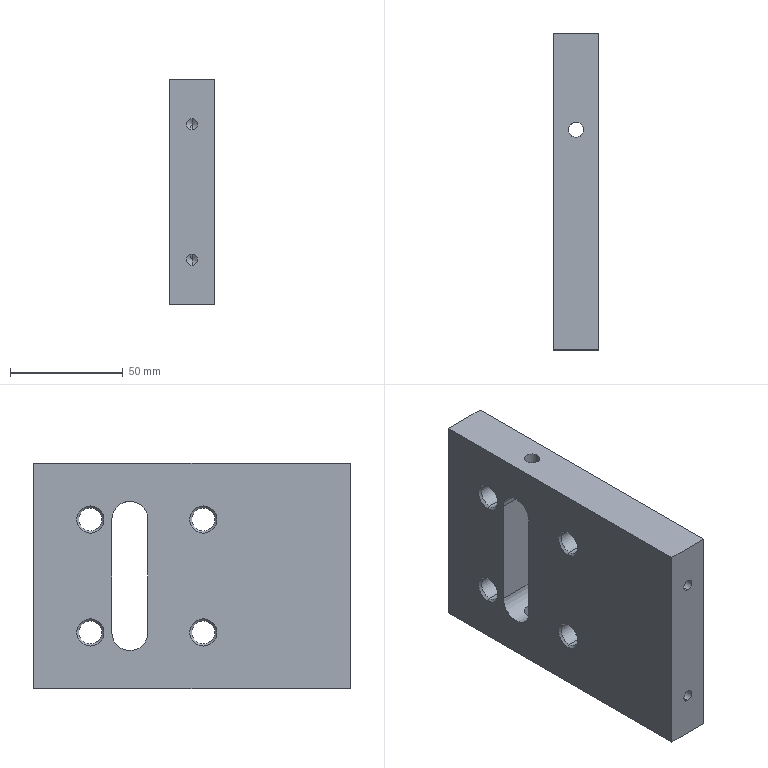Part | SolidWorks | features HoleWzd 4, Extrusion 1, ICE 1 | 1 solid | 47 faces | box 20 x 140 x 100 mm | volume 250918 mm3 | cylinder 23 | cone 16 | plane 8 | commonest cylinder face diameters 5 x8 10.2 x8 6.8 x4 16 x3
STEP:
#1=CARTESIAN_POINT('',(10.,55.,-32.5));
#2=VERTEX_POINT('',#1);
#3=CARTESIAN_POINT('',(10.,55.,-27.5));
#4=VERTEX_POINT('',#3);
#5=CARTESIAN_POINT('',(10.,55.,-30.));
#6=DIRECTION('',(0.,1.,0.));
#7=DIRECTION('',(0.,0.,1.));
#8=AXIS2_PLACEMENT_3D('',#5,#6,#7);
#9=CIRCLE('',#8,2.5);
#10=EDGE_CURVE('',#2,#4,#9,.T.);
#11=ORIENTED_EDGE('',*,*,#10,.F.);
#12=CARTESIAN_POINT('',(10.,70.,-32.5));
#13=VERTEX_POINT('',#12);
#14=CARTESIAN_POINT('',(10.,70.,-32.5));
#15=DIRECTION('',(0.,1.,0.));
#16=VECTOR('',#15,1000.);
#17=LINE('',#14,#16);
#18=EDGE_CURVE('',#2,#13,#17,.T.);
#19=ORIENTED_EDGE('',*,*,#18,.T.);
#20=CARTESIAN_POINT('',(10.,70.,-27.5));
#21=VERTEX_POINT('',#20);
#22=CARTESIAN_POINT('',(10.,70.,-30.));
#23=DIRECTION('',(0.,1.,0.));
#24=DIRECTION('',(0.,0.,1.));
#25=AXIS2_PLACEMENT_3D('',#22,#23,#24);
#26=CIRCLE('',#25,2.5);
#27=EDGE_CURVE('',#13,#21,#26,.T.);
#28=ORIENTED_EDGE('',*,*,#27,.T.);
#29=CARTESIAN_POINT('',(10.,70.,-27.5));
#30=DIRECTION('',(0.,1.,0.));
#31=VECTOR('',#30,1000.);
#32=LINE('',#29,#31);
#33=EDGE_CURVE('',#4,#21,#32,.T.);
#34=ORIENTED_EDGE('',*,*,#33,.F.);
#35=EDGE_LOOP('',(#11,#19,#28,#34));
#36=FACE_OUTER_BOUND('',#35,.T.);
#37=CARTESIAN_POINT('',(10.,70.,-30.));
#38=DIRECTION('',(0.,1.,0.));
#39=DIRECTION('',(0.,0.,1.));
#40=AXIS2_PLACEMENT_3D('',#37,#38,#39);
#41=CYLINDRICAL_SURFACE('',#40,2.5);
#42=ADVANCED_FACE('',(#36),#41,.F.);
#43=CARTESIAN_POINT('',(10.,53.498,-30.));
#44=VERTEX_POINT('',#43);
#45=CARTESIAN_POINT('',(10.,55.,-27.5));
#46=DIRECTION('',(0.,0.515,0.8572));
#47=VECTOR('',#46,1000.);
#48=LINE('',#45,#47);
#49=EDGE_CURVE('',#44,#4,#48,.T.);
#50=ORIENTED_EDGE('',*,*,#49,.F.);
#51=CARTESIAN_POINT('',(10.,55.,-32.5));
#52=DIRECTION('',(0.,0.515,-0.8572));
#53=VECTOR('',#52,1000.);
#54=LINE('',#51,#53);
#55=EDGE_CURVE('',#44,#2,#54,.T.);
#56=ORIENTED_EDGE('',*,*,#55,.T.);
#57=ORIENTED_EDGE('',*,*,#10,.T.);
#58=EDGE_LOOP('',(#50,#56,#57));
#59=FACE_OUTER_BOUND('',#58,.T.);
#60=CARTESIAN_POINT('',(10.,55.,-30.));
#61=DIRECTION('',(0.,1.,0.));
#62=DIRECTION('',(0.,0.,1.));
#63=AXIS2_PLACEMENT_3D('',#60,#61,#62);
#64=CONICAL_SURFACE('',#63,2.5,1.03);
#65=ADVANCED_FACE('',(#59),#64,.F.);
#66=CARTESIAN_POINT('',(10.,55.,27.5));
#67=VERTEX_POINT('',#66);
#68=CARTESIAN_POINT('',(10.,55.,32.5));
#69=VERTEX_POINT('',#68);
#70=CARTESIAN_POINT('',(10.,55.,30.));
#71=DIRECTION('',(0.,1.,0.));
#72=DIRECTION('',(0.,0.,1.));
#73=AXIS2_PLACEMENT_3D('',#70,#71,#72);
#74=CIRCLE('',#73,2.5);
#75=EDGE_CURVE('',#67,#69,#74,.T.);
#76=ORIENTED_EDGE('',*,*,#75,.F.);
#77=CARTESIAN_POINT('',(10.,70.,27.5));
#78=VERTEX_POINT('',#77);
#79=CARTESIAN_POINT('',(10.,70.,27.5));
#80=DIRECTION('',(0.,1.,0.));
#81=VECTOR('',#80,1000.);
#82=LINE('',#79,#81);
#83=EDGE_CURVE('',#67,#78,#82,.T.);
#84=ORIENTED_EDGE('',*,*,#83,.T.);
#85=CARTESIAN_POINT('',(10.,70.,32.5));
#86=VERTEX_POINT('',#85);
#87=CARTESIAN_POINT('',(10.,70.,30.));
#88=DIRECTION('',(0.,1.,0.));
#89=DIRECTION('',(0.,0.,1.));
#90=AXIS2_PLACEMENT_3D('',#87,#88,#89);
#91=CIRCLE('',#90,2.5);
#92=EDGE_CURVE('',#78,#86,#91,.T.);
#93=ORIENTED_EDGE('',*,*,#92,.T.);
#94=CARTESIAN_POINT('',(10.,70.,32.5));
#95=DIRECTION('',(0.,1.,0.));
#96=VECTOR('',#95,1000.);
#97=LINE('',#94,#96);
#98=EDGE_CURVE('',#69,#86,#97,.T.);
#99=ORIENTED_EDGE('',*,*,#98,.F.);
#100=EDGE_LOOP('',(#76,#84,#93,#99));
#101=FACE_OUTER_BOUND('',#100,.T.);
#102=CARTESIAN_POINT('',(10.,70.,30.));
#103=DIRECTION('',(0.,1.,0.));
#104=DIRECTION('',(0.,0.,1.));
#105=AXIS2_PLACEMENT_3D('',#102,#103,#104);
#106=CYLINDRICAL_SURFACE('',#105,2.5);
#107=ADVANCED_FACE('',(#101),#106,.F.);
#108=CARTESIAN_POINT('',(10.,53.498,30.));
#109=VERTEX_POINT('',#108);
#110=CARTESIAN_POINT('',(10.,55.,32.5));
#111=DIRECTION('',(0.,0.515,0.8572));
#112=VECTOR('',#111,1000.);
#113=LINE('',#110,#112);
#114=EDGE_CURVE('',#109,#69,#113,.T.);
#115=ORIENTED_EDGE('',*,*,#114,.F.);
#116=CARTESIAN_POINT('',(10.,55.,27.5));
#117=DIRECTION('',(0.,0.515,-0.8572));
#118=VECTOR('',#117,1000.);
#119=LINE('',#116,#118);
#120=EDGE_CURVE('',#109,#67,#119,.T.);
#121=ORIENTED_EDGE('',*,*,#120,.T.);
#122=ORIENTED_EDGE('',*,*,#75,.T.);
#123=EDGE_LOOP('',(#115,#121,#122));
#124=FACE_OUTER_BOUND('',#123,.T.);
#125=CARTESIAN_POINT('',(10.,55.,30.));
#126=DIRECTION('',(0.,1.,0.));
#127=DIRECTION('',(0.,0.,1.));
#128=AXIS2_PLACEMENT_3D('',#125,#126,#127);
#129=CONICAL_SURFACE('',#128,2.5,1.03);
#130=ADVANCED_FACE('',(#124),#129,.F.);
#131=CARTESIAN_POINT('',(0.925,45.,-30.1));
#132=VERTEX_POINT('',#131);
#133=CARTESIAN_POINT('',(0.925,45.,-19.9));
#134=VERTEX_POINT('',#133);
#135=CARTESIAN_POINT('',(0.925,45.,-25.));
#136=DIRECTION('',(-1.,0.,0.));
#137=DIRECTION('',(0.,0.,1.));
#138=AXIS2_PLACEMENT_3D('',#135,#136,#137);
#139=CIRCLE('',#138,5.1);
#140=EDGE_CURVE('',#132,#134,#139,.T.);
#141=ORIENTED_EDGE('',*,*,#140,.F.);
#142=CARTESIAN_POINT('',(0.,45.,-31.025));
#143=VERTEX_POINT('',#142);
#144=CARTESIAN_POINT('',(0.,45.,-31.025));
#145=DIRECTION('',(-0.7071,0.,-0.7071));
#146=VECTOR('',#145,1000.);
#147=LINE('',#144,#146);
#148=EDGE_CURVE('',#132,#143,#147,.T.);
#149=ORIENTED_EDGE('',*,*,#148,.T.);
#150=CARTESIAN_POINT('',(0.,45.,-18.975));
#151=VERTEX_POINT('',#150);
#152=CARTESIAN_POINT('',(0.,45.,-25.));
#153=DIRECTION('',(-1.,0.,0.));
#154=DIRECTION('',(0.,0.,1.));
#155=AXIS2_PLACEMENT_3D('',#152,#153,#154);
#156=CIRCLE('',#155,6.025);
#157=EDGE_CURVE('',#143,#151,#156,.T.);
#158=ORIENTED_EDGE('',*,*,#157,.T.);
#159=CARTESIAN_POINT('',(0.,45.,-18.975));
#160=DIRECTION('',(-0.7071,0.,0.7071));
#161=VECTOR('',#160,1000.);
#162=LINE('',#159,#161);
#163=EDGE_CURVE('',#134,#151,#162,.T.);
#164=ORIENTED_EDGE('',*,*,#163,.F.);
#165=EDGE_LOOP('',(#141,#149,#158,#164));
#166=FACE_OUTER_BOUND('',#165,.T.);
#167=CARTESIAN_POINT('',(0.,45.,-25.));
#168=DIRECTION('',(-1.,0.,0.));
#169=DIRECTION('',(0.,0.,1.));
#170=AXIS2_PLACEMENT_3D('',#167,#168,#169);
#171=CONICAL_SURFACE('',#170,6.025,0.7854);
#172=ADVANCED_FACE('',(#166),#171,.F.);
#173=CARTESIAN_POINT('',(20.,45.,-30.1));
#174=VERTEX_POINT('',#173);
#175=CARTESIAN_POINT('',(20.,45.,-19.9));
#176=VERTEX_POINT('',#175);
#177=CARTESIAN_POINT('',(20.,45.,-25.));
#178=DIRECTION('',(-1.,0.,0.));
#179=DIRECTION('',(0.,0.,1.));
#180=AXIS2_PLACEMENT_3D('',#177,#178,#179);
#181=CIRCLE('',#180,5.1);
#182=EDGE_CURVE('',#174,#176,#181,.T.);
#183=ORIENTED_EDGE('',*,*,#182,.F.);
#184=CARTESIAN_POINT('',(0.,45.,-30.1));
#185=DIRECTION('',(-1.,0.,0.));
#186=VECTOR('',#185,1000.);
#187=LINE('',#184,#186);
#188=EDGE_CURVE('',#174,#132,#187,.T.);
#189=ORIENTED_EDGE('',*,*,#188,.T.);
#190=ORIENTED_EDGE('',*,*,#140,.T.);
#191=CARTESIAN_POINT('',(0.,45.,-19.9));
#192=DIRECTION('',(-1.,0.,0.));
#193=VECTOR('',#192,1000.);
#194=LINE('',#191,#193);
#195=EDGE_CURVE('',#176,#134,#194,.T.);
#196=ORIENTED_EDGE('',*,*,#195,.F.);
#197=EDGE_LOOP('',(#183,#189,#190,#196));
#198=FACE_OUTER_BOUND('',#197,.T.);
#199=CARTESIAN_POINT('',(0.,45.,-25.));
#200=DIRECTION('',(-1.,0.,0.));
#201=DIRECTION('',(0.,0.,1.));
#202=AXIS2_PLACEMENT_3D('',#199,#200,#201);
#203=CYLINDRICAL_SURFACE('',#202,5.1);
#204=ADVANCED_FACE('',(#198),#203,.F.);
#205=CARTESIAN_POINT('',(0.925,45.,19.9));
#206=VERTEX_POINT('',#205);
#207=CARTESIAN_POINT('',(0.925,45.,30.1));
#208=VERTEX_POINT('',#207);
#209=CARTESIAN_POINT('',(0.925,45.,25.));
#210=DIRECTION('',(-1.,0.,0.));
#211=DIRECTION('',(0.,0.,1.));
#212=AXIS2_PLACEMENT_3D('',#209,#210,#211);
#213=CIRCLE('',#212,5.1);
#214=EDGE_CURVE('',#206,#208,#213,.T.);
#215=ORIENTED_EDGE('',*,*,#214,.F.);
#216=CARTESIAN_POINT('',(0.,45.,18.975));
#217=VERTEX_POINT('',#216);
#218=CARTESIAN_POINT('',(0.,45.,18.975));
#219=DIRECTION('',(-0.7071,0.,-0.7071));
#220=VECTOR('',#219,1000.);
#221=LINE('',#218,#220);
#222=EDGE_CURVE('',#206,#217,#221,.T.);
#223=ORIENTED_EDGE('',*,*,#222,.T.);
#224=CARTESIAN_POINT('',(0.,45.,31.025));
#225=VERTEX_POINT('',#224);
#226=CARTESIAN_POINT('',(0.,45.,25.));
#227=DIRECTION('',(-1.,0.,0.));
#228=DIRECTION('',(0.,0.,1.));
#229=AXIS2_PLACEMENT_3D('',#226,#227,#228);
#230=CIRCLE('',#229,6.025);
#231=EDGE_CURVE('',#217,#225,#230,.T.);
#232=ORIENTED_EDGE('',*,*,#231,.T.);
#233=CARTESIAN_POINT('',(0.,45.,31.025));
#234=DIRECTION('',(-0.7071,0.,0.7071));
#235=VECTOR('',#234,1000.);
#236=LINE('',#233,#235);
#237=EDGE_CURVE('',#208,#225,#236,.T.);
#238=ORIENTED_EDGE('',*,*,#237,.F.);
#239=EDGE_LOOP('',(#215,#223,#232,#238));
#240=FACE_OUTER_BOUND('',#239,.T.);
#241=CARTESIAN_POINT('',(0.,45.,25.));
#242=DIRECTION('',(-1.,0.,0.));
#243=DIRECTION('',(0.,0.,1.));
#244=AXIS2_PLACEMENT_3D('',#241,#242,#243);
#245=CONICAL_SURFACE('',#244,6.025,0.7854);
#246=ADVANCED_FACE('',(#240),#245,.F.);
#247=CARTESIAN_POINT('',(20.,45.,19.9));
#248=VERTEX_POINT('',#247);
#249=CARTESIAN_POINT('',(20.,45.,30.1));
#250=VERTEX_POINT('',#249);
#251=CARTESIAN_POINT('',(20.,45.,25.));
#252=DIRECTION('',(-1.,0.,0.));
#253=DIRECTION('',(0.,0.,1.));
#254=AXIS2_PLACEMENT_3D('',#251,#252,#253);
#255=CIRCLE('',#254,5.1);
#256=EDGE_CURVE('',#248,#250,#255,.T.);
#257=ORIENTED_EDGE('',*,*,#256,.F.);
#258=CARTESIAN_POINT('',(0.,45.,19.9));
#259=DIRECTION('',(-1.,0.,0.));
#260=VECTOR('',#259,1000.);
#261=LINE('',#258,#260);
#262=EDGE_CURVE('',#248,#206,#261,.T.);
#263=ORIENTED_EDGE('',*,*,#262,.T.);
#264=ORIENTED_EDGE('',*,*,#214,.T.);
#265=CARTESIAN_POINT('',(0.,45.,30.1));
#266=DIRECTION('',(-1.,0.,0.));
#267=VECTOR('',#266,1000.);
#268=LINE('',#265,#267);
#269=EDGE_CURVE('',#250,#208,#268,.T.);
#270=ORIENTED_EDGE('',*,*,#269,.F.);
#271=EDGE_LOOP('',(#257,#263,#264,#270));
#272=FACE_OUTER_BOUND('',#271,.T.);
#273=CARTESIAN_POINT('',(0.,45.,25.));
#274=DIRECTION('',(-1.,0.,0.));
#275=DIRECTION('',(0.,0.,1.));
#276=AXIS2_PLACEMENT_3D('',#273,#274,#275);
#277=CYLINDRICAL_SURFACE('',#276,5.1);
#278=ADVANCED_FACE('',(#272),#277,.F.);
#279=CARTESIAN_POINT('',(0.925,-5.,-30.1));
#280=VERTEX_POINT('',#279);
#281=CARTESIAN_POINT('',(0.925,-5.,-19.9));
#282=VERTEX_POINT('',#281);
#283=CARTESIAN_POINT('',(0.925,-5.,-25.));
#284=DIRECTION('',(-1.,0.,0.));
#285=DIRECTION('',(0.,0.,1.));
#286=AXIS2_PLACEMENT_3D('',#283,#284,#285);
#287=CIRCLE('',#286,5.1);
#288=EDGE_CURVE('',#280,#282,#287,.T.);
#289=ORIENTED_EDGE('',*,*,#288,.F.);
#290=CARTESIAN_POINT('',(0.,-5.,-31.025));
#291=VERTEX_POINT('',#290);
#292=CARTESIAN_POINT('',(0.,-5.,-31.025));
#293=DIRECTION('',(-0.7071,0.,-0.7071));
#294=VECTOR('',#293,1000.);
#295=LINE('',#292,#294);
#296=EDGE_CURVE('',#280,#291,#295,.T.);
#297=ORIENTED_EDGE('',*,*,#296,.T.);
#298=CARTESIAN_POINT('',(0.,-5.,-18.975));
#299=VERTEX_POINT('',#298);
#300=CARTESIAN_POINT('',(0.,-5.,-25.));
#301=DIRECTION('',(-1.,0.,0.));
#302=DIRECTION('',(0.,0.,1.));
#303=AXIS2_PLACEMENT_3D('',#300,#301,#302);
#304=CIRCLE('',#303,6.025);
#305=EDGE_CURVE('',#291,#299,#304,.T.);
#306=ORIENTED_EDGE('',*,*,#305,.T.);
#307=CARTESIAN_POINT('',(0.,-5.,-18.975));
#308=DIRECTION('',(-0.7071,0.,0.7071));
#309=VECTOR('',#308,1000.);
#310=LINE('',#307,#309);
#311=EDGE_CURVE('',#282,#299,#310,.T.);
#312=ORIENTED_EDGE('',*,*,#311,.F.);
#313=EDGE_LOOP('',(#289,#297,#306,#312));
#314=FACE_OUTER_BOUND('',#313,.T.);
#315=CARTESIAN_POINT('',(0.,-5.,-25.));
#316=DIRECTION('',(-1.,0.,0.));
#317=DIRECTION('',(0.,0.,1.));
#318=AXIS2_PLACEMENT_3D('',#315,#316,#317);
#319=CONICAL_SURFACE('',#318,6.025,0.7854);
#320=ADVANCED_FACE('',(#314),#319,.F.);
#321=CARTESIAN_POINT('',(20.,-5.,-30.1));
#322=VERTEX_POINT('',#321);
#323=CARTESIAN_POINT('',(20.,-5.,-19.9));
#324=VERTEX_POINT('',#323);
#325=CARTESIAN_POINT('',(20.,-5.,-25.));
#326=DIRECTION('',(-1.,0.,0.));
#327=DIRECTION('',(0.,0.,1.));
#328=AXIS2_PLACEMENT_3D('',#325,#326,#327);
#329=CIRCLE('',#328,5.1);
#330=EDGE_CURVE('',#322,#324,#329,.T.);
#331=ORIENTED_EDGE('',*,*,#330,.F.);
#332=CARTESIAN_POINT('',(0.,-5.,-30.1));
#333=DIRECTION('',(-1.,0.,0.));
#334=VECTOR('',#333,1000.);
#335=LINE('',#332,#334);
#336=EDGE_CURVE('',#322,#280,#335,.T.);
#337=ORIENTED_EDGE('',*,*,#336,.T.);
#338=ORIENTED_EDGE('',*,*,#288,.T.);
#339=CARTESIAN_POINT('',(0.,-5.,-19.9));
#340=DIRECTION('',(-1.,0.,0.));
#341=VECTOR('',#340,1000.);
#342=LINE('',#339,#341);
#343=EDGE_CURVE('',#324,#282,#342,.T.);
#344=ORIENTED_EDGE('',*,*,#343,.F.);
#345=EDGE_LOOP('',(#331,#337,#338,#344));
#346=FACE_OUTER_BOUND('',#345,.T.);
#347=CARTESIAN_POINT('',(0.,-5.,-25.));
#348=DIRECTION('',(-1.,0.,0.));
#349=DIRECTION('',(0.,0.,1.));
#350=AXIS2_PLACEMENT_3D('',#347,#348,#349);
#351=CYLINDRICAL_SURFACE('',#350,5.1);
#352=ADVANCED_FACE('',(#346),#351,.F.);
#353=CARTESIAN_POINT('',(0.925,-5.,19.9));
#354=VERTEX_POINT('',#353);
#355=CARTESIAN_POINT('',(0.925,-5.,30.1));
#356=VERTEX_POINT('',#355);
#357=CARTESIAN_POINT('',(0.925,-5.,25.));
#358=DIRECTION('',(-1.,0.,0.));
#359=DIRECTION('',(0.,0.,1.));
#360=AXIS2_PLACEMENT_3D('',#357,#358,#359);
#361=CIRCLE('',#360,5.1);
#362=EDGE_CURVE('',#354,#356,#361,.T.);
#363=ORIENTED_EDGE('',*,*,#362,.F.);
#364=CARTESIAN_POINT('',(0.,-5.,18.975));
#365=VERTEX_POINT('',#364);
#366=CARTESIAN_POINT('',(0.,-5.,18.975));
#367=DIRECTION('',(-0.7071,0.,-0.7071));
#368=VECTOR('',#367,1000.);
#369=LINE('',#366,#368);
#370=EDGE_CURVE('',#354,#365,#369,.T.);
#371=ORIENTED_EDGE('',*,*,#370,.T.);
#372=CARTESIAN_POINT('',(0.,-5.,31.025));
#373=VERTEX_POINT('',#372);
#374=CARTESIAN_POINT('',(0.,-5.,25.));
#375=DIRECTION('',(-1.,0.,0.));
#376=DIRECTION('',(0.,0.,1.));
#377=AXIS2_PLACEMENT_3D('',#374,#375,#376);
#378=CIRCLE('',#377,6.025);
#379=EDGE_CURVE('',#365,#373,#378,.T.);
#380=ORIENTED_EDGE('',*,*,#379,.T.);
#381=CARTESIAN_POINT('',(0.,-5.,31.025));
#382=DIRECTION('',(-0.7071,0.,0.7071));
#383=VECTOR('',#382,1000.);
#384=LINE('',#381,#383);
#385=EDGE_CURVE('',#356,#373,#384,.T.);
#386=ORIENTED_EDGE('',*,*,#385,.F.);
#387=EDGE_LOOP('',(#363,#371,#380,#386));
#388=FACE_OUTER_BOUND('',#387,.T.);
#389=CARTESIAN_POINT('',(0.,-5.,25.));
#390=DIRECTION('',(-1.,0.,0.));
#391=DIRECTION('',(0.,0.,1.));
#392=AXIS2_PLACEMENT_3D('',#389,#390,#391);
#393=CONICAL_SURFACE('',#392,6.025,0.7854);
#394=ADVANCED_FACE('',(#388),#393,.F.);
#395=CARTESIAN_POINT('',(20.,-5.,19.9));
#396=VERTEX_POINT('',#395);
#397=CARTESIAN_POINT('',(20.,-5.,30.1));
#398=VERTEX_POINT('',#397);
#399=CARTESIAN_POINT('',(20.,-5.,25.));
#400=DIRECTION('',(-1.,0.,0.));
#401=DIRECTION('',(0.,0.,1.));
#402=AXIS2_PLACEMENT_3D('',#399,#400,#401);
#403=CIRCLE('',#402,5.1);
#404=EDGE_CURVE('',#396,#398,#403,.T.);
#405=ORIENTED_EDGE('',*,*,#404,.F.);
#406=CARTESIAN_POINT('',(0.,-5.,19.9));
#407=DIRECTION('',(-1.,0.,0.));
#408=VECTOR('',#407,1000.);
#409=LINE('',#406,#408);
#410=EDGE_CURVE('',#396,#354,#409,.T.);
#411=ORIENTED_EDGE('',*,*,#410,.T.);
#412=ORIENTED_EDGE('',*,*,#362,.T.);
#413=CARTESIAN_POINT('',(0.,-5.,30.1));
#414=DIRECTION('',(-1.,0.,0.));
#415=VECTOR('',#414,1000.);
#416=LINE('',#413,#415);
#417=EDGE_CURVE('',#398,#356,#416,.T.);
#418=ORIENTED_EDGE('',*,*,#417,.F.);
#419=EDGE_LOOP('',(#405,#411,#412,#418));
#420=FACE_OUTER_BOUND('',#419,.T.);
#421=CARTESIAN_POINT('',(0.,-5.,25.));
#422=DIRECTION('',(-1.,0.,0.));
#423=DIRECTION('',(0.,0.,1.));
#424=AXIS2_PLACEMENT_3D('',#421,#422,#423);
#425=CYLINDRICAL_SURFACE('',#424,5.1);
#426=ADVANCED_FACE('',(#420),#425,.F.);
#427=CARTESIAN_POINT('',(6.6,27.5,-50.));
#428=VERTEX_POINT('',#427);
#429=CARTESIAN_POINT('',(13.4,27.5,-50.));
#430=VERTEX_POINT('',#429);
#431=CARTESIAN_POINT('',(10.,27.5,-50.));
#432=DIRECTION('',(0.,0.,1.));
#433=DIRECTION('',(1.,0.,0.));
#434=AXIS2_PLACEMENT_3D('',#431,#432,#433);
#435=CIRCLE('',#434,3.4);
#436=EDGE_CURVE('',#428,#430,#435,.T.);
#437=ORIENTED_EDGE('',*,*,#436,.F.);
#438=CARTESIAN_POINT('',(6.6,27.5,-33.));
#439=VERTEX_POINT('',#438);
#440=CARTESIAN_POINT('',(6.6,27.5,50.));
#441=DIRECTION('',(0.,0.,1.));
#442=VECTOR('',#441,1000.);
#443=LINE('',#440,#442);
#444=EDGE_CURVE('',#428,#439,#443,.T.);
#445=ORIENTED_EDGE('',*,*,#444,.T.);
#446=CARTESIAN_POINT('',(13.4,27.5,-33.));
#447=VERTEX_POINT('',#446);
#448=CARTESIAN_POINT('',(13.4,27.5,-33.));
#449=CARTESIAN_POINT('',(13.4,27.272,-33.));
#450=CARTESIAN_POINT('',(13.377,27.049,-32.99));
#451=CARTESIAN_POINT('',(13.289,26.611,-32.953));
#452=CARTESIAN_POINT('',(13.223,26.393,-32.926));
#453=CARTESIAN_POINT('',(13.051,25.983,-32.858));
#454=CARTESIAN_POINT('',(12.946,25.788,-32.817));
#455=CARTESIAN_POINT('',(12.699,25.42,-32.727));
#456=CARTESIAN_POINT('',(12.557,25.249,-32.678));
#457=CARTESIAN_POINT('',(12.247,24.939,-32.581));
#458=CARTESIAN_POINT('',(12.077,24.799,-32.531));
#459=CARTESIAN_POINT('',(11.708,24.552,-32.438));
#460=CARTESIAN_POINT('',(11.514,24.448,-32.395));
#461=CARTESIAN_POINT('',(11.107,24.278,-32.323));
#462=CARTESIAN_POINT('',(10.89,24.211,-32.293));
#463=CARTESIAN_POINT('',(10.45,24.122,-32.252));
#464=CARTESIAN_POINT('',(10.227,24.1,-32.242));
#465=CARTESIAN_POINT('',(9.777,24.1,-32.241));
#466=CARTESIAN_POINT('',(9.549,24.123,-32.252));
#467=CARTESIAN_POINT('',(9.111,24.211,-32.293));
#468=CARTESIAN_POINT('',(8.896,24.276,-32.322));
#469=CARTESIAN_POINT('',(8.483,24.449,-32.396));
#470=CARTESIAN_POINT('',(8.289,24.554,-32.439));
#471=CARTESIAN_POINT('',(7.923,24.799,-32.531));
#472=CARTESIAN_POINT('',(7.75,24.941,-32.582));
#473=CARTESIAN_POINT('',(7.44,25.252,-32.679));
#474=CARTESIAN_POINT('',(7.301,25.421,-32.727));
#475=CARTESIAN_POINT('',(7.054,25.789,-32.817));
#476=CARTESIAN_POINT('',(6.948,25.986,-32.858));
#477=CARTESIAN_POINT('',(6.777,26.395,-32.926));
#478=CARTESIAN_POINT('',(6.711,26.608,-32.953));
#479=CARTESIAN_POINT('',(6.622,27.052,-32.991));
#480=CARTESIAN_POINT('',(6.6,27.276,-33.));
#481=CARTESIAN_POINT('',(6.6,27.5,-33.));
#482=B_SPLINE_CURVE_WITH_KNOTS('',3,(#448,#449,#450,#451,#452,#453,#454,#455,#456,#457,#458,#459,#460,#461,#462,#463,#464,#465,#466,#467,#468,#469,#470,#471,#472,#473,#474,#475,#476,#477,#478,#479,#480,#481),.UNSPECIFIED.,.F.,.F.,(4,2,2,2,2,2,2,2,2,2,2,2,2,2,2,2,4),(0.,0.0006725,0.001345,0.002017,0.00269,0.003362,0.004035,0.004707,0.00538,0.006052,0.006725,0.007397,0.00807,0.008742,0.009415,0.01009,0.01076),.UNSPECIFIED.);
#483=EDGE_CURVE('',#447,#439,#482,.T.);
#484=ORIENTED_EDGE('',*,*,#483,.F.);
#485=CARTESIAN_POINT('',(13.4,27.5,50.));
#486=DIRECTION('',(0.,0.,1.));
#487=VECTOR('',#486,1000.);
#488=LINE('',#485,#487);
#489=EDGE_CURVE('',#430,#447,#488,.T.);
#490=ORIENTED_EDGE('',*,*,#489,.F.);
#491=EDGE_LOOP('',(#437,#445,#484,#490));
#492=FACE_OUTER_BOUND('',#491,.T.);
#493=CARTESIAN_POINT('',(10.,27.5,50.));
#494=DIRECTION('',(0.,0.,1.));
#495=DIRECTION('',(1.,0.,0.));
#496=AXIS2_PLACEMENT_3D('',#493,#494,#495);
#497=CYLINDRICAL_SURFACE('',#496,3.4);
#498=ADVANCED_FACE('',(#492),#497,.F.);
#499=CARTESIAN_POINT('',(6.6,27.5,33.));
#500=VERTEX_POINT('',#499);
#501=CARTESIAN_POINT('',(13.4,27.5,33.));
#502=VERTEX_POINT('',#501);
#503=CARTESIAN_POINT('',(6.6,27.5,33.));
#504=CARTESIAN_POINT('',(6.6,27.276,33.));
#505=CARTESIAN_POINT('',(6.623,27.049,32.99));
#506=CARTESIAN_POINT('',(6.711,26.608,32.953));
#507=CARTESIAN_POINT('',(6.777,26.395,32.926));
#508=CARTESIAN_POINT('',(6.949,25.983,32.858));
#509=CARTESIAN_POINT('',(7.055,25.786,32.816));
#510=CARTESIAN_POINT('',(7.301,25.421,32.727));
#511=CARTESIAN_POINT('',(7.442,25.25,32.679));
#512=CARTESIAN_POINT('',(7.754,24.938,32.58));
#513=CARTESIAN_POINT('',(7.924,24.799,32.531));
#514=CARTESIAN_POINT('',(8.288,24.554,32.439));
#515=CARTESIAN_POINT('',(8.486,24.447,32.395));
#516=CARTESIAN_POINT('',(8.896,24.277,32.322));
#517=CARTESIAN_POINT('',(9.108,24.212,32.293));
#518=CARTESIAN_POINT('',(9.547,24.123,32.252));
#519=CARTESIAN_POINT('',(9.775,24.1,32.242));
#520=CARTESIAN_POINT('',(10.223,24.1,32.242));
#521=CARTESIAN_POINT('',(10.446,24.122,32.252));
#522=CARTESIAN_POINT('',(10.891,24.211,32.293));
#523=CARTESIAN_POINT('',(11.104,24.276,32.322));
#524=CARTESIAN_POINT('',(11.513,24.447,32.395));
#525=CARTESIAN_POINT('',(11.711,24.554,32.439));
#526=CARTESIAN_POINT('',(12.077,24.799,32.531));
#527=CARTESIAN_POINT('',(12.247,24.938,32.581));
#528=CARTESIAN_POINT('',(12.559,25.25,32.679));
#529=CARTESIAN_POINT('',(12.7,25.422,32.728));
#530=CARTESIAN_POINT('',(12.945,25.786,32.817));
#531=CARTESIAN_POINT('',(13.05,25.982,32.857));
#532=CARTESIAN_POINT('',(13.223,26.396,32.926));
#533=CARTESIAN_POINT('',(13.289,26.608,32.953));
#534=CARTESIAN_POINT('',(13.377,27.046,32.99));
#535=CARTESIAN_POINT('',(13.4,27.273,33.));
#536=CARTESIAN_POINT('',(13.4,27.5,33.));
#537=B_SPLINE_CURVE_WITH_KNOTS('',3,(#503,#504,#505,#506,#507,#508,#509,#510,#511,#512,#513,#514,#515,#516,#517,#518,#519,#520,#521,#522,#523,#524,#525,#526,#527,#528,#529,#530,#531,#532,#533,#534,#535,#536),.UNSPECIFIED.,.F.,.F.,(4,2,2,2,2,2,2,2,2,2,2,2,2,2,2,2,4),(0.01076,0.01143,0.0121,0.01278,0.01345,0.01412,0.01479,0.01546,0.01613,0.01681,0.01748,0.01815,0.01882,0.01949,0.02017,0.02084,0.02151),.UNSPECIFIED.);
#538=EDGE_CURVE('',#500,#502,#537,.T.);
#539=ORIENTED_EDGE('',*,*,#538,.F.);
#540=CARTESIAN_POINT('',(6.6,27.5,50.));
#541=VERTEX_POINT('',#540);
#542=CARTESIAN_POINT('',(6.6,27.5,50.));
#543=DIRECTION('',(0.,0.,1.));
#544=VECTOR('',#543,1000.);
#545=LINE('',#542,#544);
#546=EDGE_CURVE('',#500,#541,#545,.T.);
#547=ORIENTED_EDGE('',*,*,#546,.T.);
#548=CARTESIAN_POINT('',(13.4,27.5,50.));
#549=VERTEX_POINT('',#548);
#550=CARTESIAN_POINT('',(10.,27.5,50.));
#551=DIRECTION('',(0.,0.,1.));
#552=DIRECTION('',(1.,0.,0.));
#553=AXIS2_PLACEMENT_3D('',#550,#551,#552);
#554=CIRCLE('',#553,3.4);
#555=EDGE_CURVE('',#541,#549,#554,.T.);
#556=ORIENTED_EDGE('',*,*,#555,.T.);
#557=CARTESIAN_POINT('',(13.4,27.5,50.));
#558=DIRECTION('',(0.,0.,1.));
#559=VECTOR('',#558,1000.);
#560=LINE('',#557,#559);
#561=EDGE_CURVE('',#502,#549,#560,.T.);
#562=ORIENTED_EDGE('',*,*,#561,.F.);
#563=EDGE_LOOP('',(#539,#547,#556,#562));
#564=FACE_OUTER_BOUND('',#563,.T.);
#565=CARTESIAN_POINT('',(10.,27.5,50.));
#566=DIRECTION('',(0.,0.,1.));
#567=DIRECTION('',(1.,0.,0.));
#568=AXIS2_PLACEMENT_3D('',#565,#566,#567);
#569=CYLINDRICAL_SURFACE('',#568,3.4);
#570=ADVANCED_FACE('',(#564),#569,.F.);
#571=CARTESIAN_POINT('',(20.,27.5,33.));
#572=VERTEX_POINT('',#571);
#573=CARTESIAN_POINT('',(20.,35.5,25.));
#574=VERTEX_POINT('',#573);
#575=CARTESIAN_POINT('',(20.,27.5,25.));
#576=DIRECTION('',(-1.,0.,0.));
#577=DIRECTION('',(0.,0.,1.));
#578=AXIS2_PLACEMENT_3D('',#575,#576,#577);
#579=CIRCLE('',#578,8.);
#580=EDGE_CURVE('',#572,#574,#579,.T.);
#581=ORIENTED_EDGE('',*,*,#580,.F.);
#582=CARTESIAN_POINT('',(20.,27.5,33.));
#583=DIRECTION('',(-1.,0.,0.));
#584=VECTOR('',#583,1000.);
#585=LINE('',#582,#584);
#586=EDGE_CURVE('',#572,#502,#585,.T.);
#587=ORIENTED_EDGE('',*,*,#586,.T.);
#588=CARTESIAN_POINT('',(13.4,27.5,33.));
#589=CARTESIAN_POINT('',(13.4,27.728,33.));
#590=CARTESIAN_POINT('',(13.377,27.951,32.99));
#591=CARTESIAN_POINT('',(13.289,28.389,32.953));
#592=CARTESIAN_POINT('',(13.223,28.607,32.926));
#593=CARTESIAN_POINT('',(13.051,29.017,32.858));
#594=CARTESIAN_POINT('',(12.946,29.212,32.817));
#595=CARTESIAN_POINT('',(12.699,29.58,32.727));
#596=CARTESIAN_POINT('',(12.557,29.751,32.678));
#597=CARTESIAN_POINT('',(12.247,30.061,32.581));
#598=CARTESIAN_POINT('',(12.077,30.201,32.531));
#599=CARTESIAN_POINT('',(11.708,30.448,32.438));
#600=CARTESIAN_POINT('',(11.514,30.552,32.395));
#601=CARTESIAN_POINT('',(11.107,30.722,32.323));
#602=CARTESIAN_POINT('',(10.89,30.789,32.293));
#603=CARTESIAN_POINT('',(10.45,30.878,32.252));
#604=CARTESIAN_POINT('',(10.227,30.9,32.242));
#605=CARTESIAN_POINT('',(9.777,30.9,32.241));
#606=CARTESIAN_POINT('',(9.549,30.877,32.252));
#607=CARTESIAN_POINT('',(9.111,30.789,32.293));
#608=CARTESIAN_POINT('',(8.896,30.724,32.322));
#609=CARTESIAN_POINT('',(8.483,30.551,32.396));
#610=CARTESIAN_POINT('',(8.289,30.446,32.439));
#611=CARTESIAN_POINT('',(7.923,30.201,32.531));
#612=CARTESIAN_POINT('',(7.75,30.059,32.582));
#613=CARTESIAN_POINT('',(7.44,29.748,32.679));
#614=CARTESIAN_POINT('',(7.301,29.579,32.727));
#615=CARTESIAN_POINT('',(7.054,29.211,32.817));
#616=CARTESIAN_POINT('',(6.948,29.014,32.858));
#617=CARTESIAN_POINT('',(6.777,28.605,32.926));
#618=CARTESIAN_POINT('',(6.711,28.392,32.953));
#619=CARTESIAN_POINT('',(6.622,27.948,32.991));
#620=CARTESIAN_POINT('',(6.6,27.724,33.));
#621=CARTESIAN_POINT('',(6.6,27.5,33.));
#622=B_SPLINE_CURVE_WITH_KNOTS('',3,(#588,#589,#590,#591,#592,#593,#594,#595,#596,#597,#598,#599,#600,#601,#602,#603,#604,#605,#606,#607,#608,#609,#610,#611,#612,#613,#614,#615,#616,#617,#618,#619,#620,#621),.UNSPECIFIED.,.F.,.F.,(4,2,2,2,2,2,2,2,2,2,2,2,2,2,2,2,4),(0.,0.0006725,0.001345,0.002017,0.00269,0.003362,0.004035,0.004707,0.00538,0.006052,0.006725,0.007397,0.00807,0.008742,0.009415,0.01009,0.01076),.UNSPECIFIED.);
#623=EDGE_CURVE('',#502,#500,#622,.T.);
#624=ORIENTED_EDGE('',*,*,#623,.T.);
#625=CARTESIAN_POINT('',(0.,27.5,33.));
#626=VERTEX_POINT('',#625);
#627=CARTESIAN_POINT('',(20.,27.5,33.));
#628=DIRECTION('',(-1.,0.,0.));
#629=VECTOR('',#628,1000.);
#630=LINE('',#627,#629);
#631=EDGE_CURVE('',#500,#626,#630,.T.);
#632=ORIENTED_EDGE('',*,*,#631,.T.);
#633=CARTESIAN_POINT('',(0.,35.5,25.));
#634=VERTEX_POINT('',#633);
#635=CARTESIAN_POINT('',(0.,27.5,25.));
#636=DIRECTION('',(-1.,0.,0.));
#637=DIRECTION('',(0.,0.,1.));
#638=AXIS2_PLACEMENT_3D('',#635,#636,#637);
#639=CIRCLE('',#638,8.);
#640=EDGE_CURVE('',#626,#634,#639,.T.);
#641=ORIENTED_EDGE('',*,*,#640,.T.);
#642=CARTESIAN_POINT('',(20.,35.5,25.));
#643=DIRECTION('',(-1.,0.,0.));
#644=VECTOR('',#643,1000.);
#645=LINE('',#642,#644);
#646=EDGE_CURVE('',#574,#634,#645,.T.);
#647=ORIENTED_EDGE('',*,*,#646,.F.);
#648=EDGE_LOOP('',(#581,#587,#624,#632,#641,#647));
#649=FACE_OUTER_BOUND('',#648,.T.);
#650=CARTESIAN_POINT('',(20.,27.5,25.));
#651=DIRECTION('',(-1.,0.,0.));
#652=DIRECTION('',(0.,0.,1.));
#653=AXIS2_PLACEMENT_3D('',#650,#651,#652);
#654=CYLINDRICAL_SURFACE('',#653,8.);
#655=ADVANCED_FACE('',(#649),#654,.F.);
#656=CARTESIAN_POINT('',(10.,-55.,-27.5));
#657=VERTEX_POINT('',#656);
#658=CARTESIAN_POINT('',(10.,-55.,-32.5));
#659=VERTEX_POINT('',#658);
#660=CARTESIAN_POINT('',(10.,-55.,-30.));
#661=DIRECTION('',(0.,-1.,0.));
#662=DIRECTION('',(0.,0.,-1.));
#663=AXIS2_PLACEMENT_3D('',#660,#661,#662);
#664=CIRCLE('',#663,2.5);
#665=EDGE_CURVE('',#657,#659,#664,.T.);
#666=ORIENTED_EDGE('',*,*,#665,.F.);
#667=CARTESIAN_POINT('',(10.,-70.,-27.5));
#668=VERTEX_POINT('',#667);
#669=CARTESIAN_POINT('',(10.,-70.,-27.5));
#670=DIRECTION('',(0.,-1.,0.));
#671=VECTOR('',#670,1000.);
#672=LINE('',#669,#671);
#673=EDGE_CURVE('',#657,#668,#672,.T.);
#674=ORIENTED_EDGE('',*,*,#673,.T.);
#675=CARTESIAN_POINT('',(10.,-70.,-32.5));
#676=VERTEX_POINT('',#675);
#677=CARTESIAN_POINT('',(10.,-70.,-30.));
#678=DIRECTION('',(0.,-1.,0.));
#679=DIRECTION('',(0.,0.,-1.));
#680=AXIS2_PLACEMENT_3D('',#677,#678,#679);
#681=CIRCLE('',#680,2.5);
#682=EDGE_CURVE('',#668,#676,#681,.T.);
#683=ORIENTED_EDGE('',*,*,#682,.T.);
#684=CARTESIAN_POINT('',(10.,-70.,-32.5));
#685=DIRECTION('',(0.,-1.,0.));
#686=VECTOR('',#685,1000.);
#687=LINE('',#684,#686);
#688=EDGE_CURVE('',#659,#676,#687,.T.);
#689=ORIENTED_EDGE('',*,*,#688,.F.);
#690=EDGE_LOOP('',(#666,#674,#683,#689));
#691=FACE_OUTER_BOUND('',#690,.T.);
#692=CARTESIAN_POINT('',(10.,-70.,-30.));
#693=DIRECTION('',(0.,-1.,0.));
#694=DIRECTION('',(0.,0.,-1.));
#695=AXIS2_PLACEMENT_3D('',#692,#693,#694);
#696=CYLINDRICAL_SURFACE('',#695,2.5);
#697=ADVANCED_FACE('',(#691),#696,.F.);
#698=CARTESIAN_POINT('',(10.,-53.498,-30.));
#699=VERTEX_POINT('',#698);
#700=CARTESIAN_POINT('',(10.,-55.,-32.5));
#701=DIRECTION('',(0.,-0.515,-0.8572));
#702=VECTOR('',#701,1000.);
#703=LINE('',#700,#702);
#704=EDGE_CURVE('',#699,#659,#703,.T.);
#705=ORIENTED_EDGE('',*,*,#704,.F.);
#706=CARTESIAN_POINT('',(10.,-55.,-27.5));
#707=DIRECTION('',(0.,-0.515,0.8572));
#708=VECTOR('',#707,1000.);
#709=LINE('',#706,#708);
#710=EDGE_CURVE('',#699,#657,#709,.T.);
#711=ORIENTED_EDGE('',*,*,#710,.T.);
#712=ORIENTED_EDGE('',*,*,#665,.T.);
#713=EDGE_LOOP('',(#705,#711,#712));
#714=FACE_OUTER_BOUND('',#713,.T.);
#715=CARTESIAN_POINT('',(10.,-55.,-30.));
#716=DIRECTION('',(0.,-1.,0.));
#717=DIRECTION('',(0.,0.,-1.));
#718=AXIS2_PLACEMENT_3D('',#715,#716,#717);
#719=CONICAL_SURFACE('',#718,2.5,1.03);
#720=ADVANCED_FACE('',(#714),#719,.F.);
#721=CARTESIAN_POINT('',(10.,-55.,32.5));
#722=VERTEX_POINT('',#721);
#723=CARTESIAN_POINT('',(10.,-55.,27.5));
#724=VERTEX_POINT('',#723);
#725=CARTESIAN_POINT('',(10.,-55.,30.));
#726=DIRECTION('',(0.,-1.,0.));
#727=DIRECTION('',(0.,0.,-1.));
#728=AXIS2_PLACEMENT_3D('',#725,#726,#727);
#729=CIRCLE('',#728,2.5);
#730=EDGE_CURVE('',#722,#724,#729,.T.);
#731=ORIENTED_EDGE('',*,*,#730,.F.);
#732=CARTESIAN_POINT('',(10.,-70.,32.5));
#733=VERTEX_POINT('',#732);
#734=CARTESIAN_POINT('',(10.,-70.,32.5));
#735=DIRECTION('',(0.,-1.,0.));
#736=VECTOR('',#735,1000.);
#737=LINE('',#734,#736);
#738=EDGE_CURVE('',#722,#733,#737,.T.);
#739=ORIENTED_EDGE('',*,*,#738,.T.);
#740=CARTESIAN_POINT('',(10.,-70.,27.5));
#741=VERTEX_POINT('',#740);
#742=CARTESIAN_POINT('',(10.,-70.,30.));
#743=DIRECTION('',(0.,-1.,0.));
#744=DIRECTION('',(0.,0.,-1.));
#745=AXIS2_PLACEMENT_3D('',#742,#743,#744);
#746=CIRCLE('',#745,2.5);
#747=EDGE_CURVE('',#733,#741,#746,.T.);
#748=ORIENTED_EDGE('',*,*,#747,.T.);
#749=CARTESIAN_POINT('',(10.,-70.,27.5));
#750=DIRECTION('',(0.,-1.,0.));
#751=VECTOR('',#750,1000.);
#752=LINE('',#749,#751);
#753=EDGE_CURVE('',#724,#741,#752,.T.);
#754=ORIENTED_EDGE('',*,*,#753,.F.);
#755=EDGE_LOOP('',(#731,#739,#748,#754));
#756=FACE_OUTER_BOUND('',#755,.T.);
#757=CARTESIAN_POINT('',(10.,-70.,30.));
#758=DIRECTION('',(0.,-1.,0.));
#759=DIRECTION('',(0.,0.,-1.));
#760=AXIS2_PLACEMENT_3D('',#757,#758,#759);
#761=CYLINDRICAL_SURFACE('',#760,2.5);
#762=ADVANCED_FACE('',(#756),#761,.F.);
#763=CARTESIAN_POINT('',(10.,-53.498,30.));
#764=VERTEX_POINT('',#763);
#765=CARTESIAN_POINT('',(10.,-55.,27.5));
#766=DIRECTION('',(0.,-0.515,-0.8572));
#767=VECTOR('',#766,1000.);
#768=LINE('',#765,#767);
#769=EDGE_CURVE('',#764,#724,#768,.T.);
#770=ORIENTED_EDGE('',*,*,#769,.F.);
#771=CARTESIAN_POINT('',(10.,-55.,32.5));
#772=DIRECTION('',(0.,-0.515,0.8572));
#773=VECTOR('',#772,1000.);
#774=LINE('',#771,#773);
#775=EDGE_CURVE('',#764,#722,#774,.T.);
#776=ORIENTED_EDGE('',*,*,#775,.T.);
#777=ORIENTED_EDGE('',*,*,#730,.T.);
#778=EDGE_LOOP('',(#770,#776,#777));
#779=FACE_OUTER_BOUND('',#778,.T.);
#780=CARTESIAN_POINT('',(10.,-55.,30.));
#781=DIRECTION('',(0.,-1.,0.));
#782=DIRECTION('',(0.,0.,-1.));
#783=AXIS2_PLACEMENT_3D('',#780,#781,#782);
#784=CONICAL_SURFACE('',#783,2.5,1.03);
#785=ADVANCED_FACE('',(#779),#784,.F.);
#786=CARTESIAN_POINT('',(10.,27.5,-50.));
#787=DIRECTION('',(0.,0.,1.));
#788=DIRECTION('',(1.,0.,0.));
#789=AXIS2_PLACEMENT_3D('',#786,#787,#788);
#790=CIRCLE('',#789,3.4);
#791=EDGE_CURVE('',#430,#428,#790,.T.);
#792=ORIENTED_EDGE('',*,*,#791,.T.);
#793=ORIENTED_EDGE('',*,*,#436,.T.);
#794=EDGE_LOOP('',(#792,#793));
#795=FACE_BOUND('',#794,.T.);
#796=CARTESIAN_POINT('',(0.,-70.,-50.));
#797=VERTEX_POINT('',#796);
#798=CARTESIAN_POINT('',(0.,70.,-50.));
#799=VERTEX_POINT('',#798);
#800=CARTESIAN_POINT('',(0.,70.,-50.));
#801=DIRECTION('',(0.,1.,0.));
#802=VECTOR('',#801,1000.);
#803=LINE('',#800,#802);
#804=EDGE_CURVE('',#797,#799,#803,.T.);
#805=ORIENTED_EDGE('',*,*,#804,.T.);
#806=CARTESIAN_POINT('',(20.,70.,-50.));
#807=VERTEX_POINT('',#806);
#808=CARTESIAN_POINT('',(20.,70.,-50.));
#809=DIRECTION('',(-1.,0.,0.));
#810=VECTOR('',#809,1000.);
#811=LINE('',#808,#810);
#812=EDGE_CURVE('',#807,#799,#811,.T.);
#813=ORIENTED_EDGE('',*,*,#812,.F.);
#814=CARTESIAN_POINT('',(20.,-70.,-50.));
#815=VERTEX_POINT('',#814);
#816=CARTESIAN_POINT('',(20.,70.,-50.));
#817=DIRECTION('',(0.,1.,0.));
#818=VECTOR('',#817,1000.);
#819=LINE('',#816,#818);
#820=EDGE_CURVE('',#815,#807,#819,.T.);
#821=ORIENTED_EDGE('',*,*,#820,.F.);
#822=CARTESIAN_POINT('',(20.,-70.,-50.));
#823=DIRECTION('',(-1.,0.,0.));
#824=VECTOR('',#823,1000.);
#825=LINE('',#822,#824);
#826=EDGE_CURVE('',#815,#797,#825,.T.);
#827=ORIENTED_EDGE('',*,*,#826,.T.);
#828=EDGE_LOOP('',(#805,#813,#821,#827));
#829=FACE_OUTER_BOUND('',#828,.T.);
#830=CARTESIAN_POINT('',(20.,70.,-50.));
#831=DIRECTION('',(0.,0.,1.));
#832=DIRECTION('',(0.,-1.,0.));
#833=AXIS2_PLACEMENT_3D('',#830,#831,#832);
#834=PLANE('',#833);
#835=ADVANCED_FACE('',(#795,#829),#834,.F.);
#836=CARTESIAN_POINT('',(10.,70.,-30.));
#837=DIRECTION('',(0.,1.,0.));
#838=DIRECTION('',(0.,0.,1.));
#839=AXIS2_PLACEMENT_3D('',#836,#837,#838);
#840=CIRCLE('',#839,2.5);
#841=EDGE_CURVE('',#21,#13,#840,.T.);
#842=ORIENTED_EDGE('',*,*,#841,.F.);
#843=ORIENTED_EDGE('',*,*,#27,.F.);
#844=EDGE_LOOP('',(#842,#843));
#845=FACE_BOUND('',#844,.T.);
#846=CARTESIAN_POINT('',(10.,70.,30.));
#847=DIRECTION('',(0.,1.,0.));
#848=DIRECTION('',(0.,0.,1.));
#849=AXIS2_PLACEMENT_3D('',#846,#847,#848);
#850=CIRCLE('',#849,2.5);
#851=EDGE_CURVE('',#86,#78,#850,.T.);
#852=ORIENTED_EDGE('',*,*,#851,.F.);
#853=ORIENTED_EDGE('',*,*,#92,.F.);
#854=EDGE_LOOP('',(#852,#853));
#855=FACE_BOUND('',#854,.T.);
#856=CARTESIAN_POINT('',(0.,70.,50.));
#857=VERTEX_POINT('',#856);
#858=CARTESIAN_POINT('',(0.,70.,50.));
#859=DIRECTION('',(0.,0.,1.));
#860=VECTOR('',#859,1000.);
#861=LINE('',#858,#860);
#862=EDGE_CURVE('',#799,#857,#861,.T.);
#863=ORIENTED_EDGE('',*,*,#862,.T.);
#864=CARTESIAN_POINT('',(20.,70.,50.));
#865=VERTEX_POINT('',#864);
#866=CARTESIAN_POINT('',(20.,70.,50.));
#867=DIRECTION('',(-1.,0.,0.));
#868=VECTOR('',#867,1000.);
#869=LINE('',#866,#868);
#870=EDGE_CURVE('',#865,#857,#869,.T.);
#871=ORIENTED_EDGE('',*,*,#870,.F.);
#872=CARTESIAN_POINT('',(20.,70.,50.));
#873=DIRECTION('',(0.,0.,1.));
#874=VECTOR('',#873,1000.);
#875=LINE('',#872,#874);
#876=EDGE_CURVE('',#807,#865,#875,.T.);
#877=ORIENTED_EDGE('',*,*,#876,.F.);
#878=ORIENTED_EDGE('',*,*,#812,.T.);
#879=EDGE_LOOP('',(#863,#871,#877,#878));
#880=FACE_OUTER_BOUND('',#879,.T.);
#881=CARTESIAN_POINT('',(20.,70.,50.));
#882=DIRECTION('',(0.,-1.,0.));
#883=DIRECTION('',(0.,0.,-1.));
#884=AXIS2_PLACEMENT_3D('',#881,#882,#883);
#885=PLANE('',#884);
#886=ADVANCED_FACE('',(#845,#855,#880),#885,.F.);
#887=CARTESIAN_POINT('',(10.,27.5,50.));
#888=DIRECTION('',(0.,0.,1.));
#889=DIRECTION('',(1.,0.,0.));
#890=AXIS2_PLACEMENT_3D('',#887,#888,#889);
#891=CIRCLE('',#890,3.4);
#892=EDGE_CURVE('',#549,#541,#891,.T.);
#893=ORIENTED_EDGE('',*,*,#892,.F.);
#894=ORIENTED_EDGE('',*,*,#555,.F.);
#895=EDGE_LOOP('',(#893,#894));
#896=FACE_BOUND('',#895,.T.);
#897=CARTESIAN_POINT('',(0.,-70.,50.));
#898=VERTEX_POINT('',#897);
#899=CARTESIAN_POINT('',(0.,70.,50.));
#900=DIRECTION('',(0.,-1.,0.));
#901=VECTOR('',#900,1000.);
#902=LINE('',#899,#901);
#903=EDGE_CURVE('',#857,#898,#902,.T.);
#904=ORIENTED_EDGE('',*,*,#903,.T.);
#905=CARTESIAN_POINT('',(20.,-70.,50.));
#906=VERTEX_POINT('',#905);
#907=CARTESIAN_POINT('',(20.,-70.,50.));
#908=DIRECTION('',(-1.,0.,0.));
#909=VECTOR('',#908,1000.);
#910=LINE('',#907,#909);
#911=EDGE_CURVE('',#906,#898,#910,.T.);
#912=ORIENTED_EDGE('',*,*,#911,.F.);
#913=CARTESIAN_POINT('',(20.,70.,50.));
#914=DIRECTION('',(0.,-1.,0.));
#915=VECTOR('',#914,1000.);
#916=LINE('',#913,#915);
#917=EDGE_CURVE('',#865,#906,#916,.T.);
#918=ORIENTED_EDGE('',*,*,#917,.F.);
#919=ORIENTED_EDGE('',*,*,#870,.T.);
#920=EDGE_LOOP('',(#904,#912,#918,#919));
#921=FACE_OUTER_BOUND('',#920,.T.);
#922=CARTESIAN_POINT('',(20.,70.,50.));
#923=DIRECTION('',(0.,0.,-1.));
#924=DIRECTION('',(0.,1.,0.));
#925=AXIS2_PLACEMENT_3D('',#922,#923,#924);
#926=PLANE('',#925);
#927=ADVANCED_FACE('',(#896,#921),#926,.F.);
#928=CARTESIAN_POINT('',(10.,-70.,-30.));
#929=DIRECTION('',(0.,-1.,0.));
#930=DIRECTION('',(0.,0.,-1.));
#931=AXIS2_PLACEMENT_3D('',#928,#929,#930);
#932=CIRCLE('',#931,2.5);
#933=EDGE_CURVE('',#676,#668,#932,.T.);
#934=ORIENTED_EDGE('',*,*,#933,.F.);
#935=ORIENTED_EDGE('',*,*,#682,.F.);
#936=EDGE_LOOP('',(#934,#935));
#937=FACE_BOUND('',#936,.T.);
#938=CARTESIAN_POINT('',(10.,-70.,30.));
#939=DIRECTION('',(0.,-1.,0.));
#940=DIRECTION('',(0.,0.,-1.));
#941=AXIS2_PLACEMENT_3D('',#938,#939,#940);
#942=CIRCLE('',#941,2.5);
#943=EDGE_CURVE('',#741,#733,#942,.T.);
#944=ORIENTED_EDGE('',*,*,#943,.F.);
#945=ORIENTED_EDGE('',*,*,#747,.F.);
#946=EDGE_LOOP('',(#944,#945));
#947=FACE_BOUND('',#946,.T.);
#948=CARTESIAN_POINT('',(0.,-70.,50.));
#949=DIRECTION('',(0.,0.,-1.));
#950=VECTOR('',#949,1000.);
#951=LINE('',#948,#950);
#952=EDGE_CURVE('',#898,#797,#951,.T.);
#953=ORIENTED_EDGE('',*,*,#952,.T.);
#954=ORIENTED_EDGE('',*,*,#826,.F.);
#955=CARTESIAN_POINT('',(20.,-70.,50.));
#956=DIRECTION('',(0.,0.,-1.));
#957=VECTOR('',#956,1000.);
#958=LINE('',#955,#957);
#959=EDGE_CURVE('',#906,#815,#958,.T.);
#960=ORIENTED_EDGE('',*,*,#959,.F.);
#961=ORIENTED_EDGE('',*,*,#911,.T.);
#962=EDGE_LOOP('',(#953,#954,#960,#961));
#963=FACE_OUTER_BOUND('',#962,.T.);
#964=CARTESIAN_POINT('',(20.,-70.,50.));
#965=DIRECTION('',(0.,1.,0.));
#966=DIRECTION('',(0.,0.,1.));
#967=AXIS2_PLACEMENT_3D('',#964,#965,#966);
#968=PLANE('',#967);
#969=ADVANCED_FACE('',(#937,#947,#963),#968,.F.);
#970=CARTESIAN_POINT('',(20.,45.,-25.));
#971=DIRECTION('',(-1.,0.,0.));
#972=DIRECTION('',(0.,0.,1.));
#973=AXIS2_PLACEMENT_3D('',#970,#971,#972);
#974=CIRCLE('',#973,5.1);
#975=EDGE_CURVE('',#176,#174,#974,.T.);
#976=ORIENTED_EDGE('',*,*,#975,.T.);
#977=ORIENTED_EDGE('',*,*,#182,.T.);
#978=EDGE_LOOP('',(#976,#977));
#979=FACE_BOUND('',#978,.T.);
#980=CARTESIAN_POINT('',(20.,45.,25.));
#981=DIRECTION('',(-1.,0.,0.));
#982=DIRECTION('',(0.,0.,1.));
#983=AXIS2_PLACEMENT_3D('',#980,#981,#982);
#984=CIRCLE('',#983,5.1);
#985=EDGE_CURVE('',#250,#248,#984,.T.);
#986=ORIENTED_EDGE('',*,*,#985,.T.);
#987=ORIENTED_EDGE('',*,*,#256,.T.);
#988=EDGE_LOOP('',(#986,#987));
#989=FACE_BOUND('',#988,.T.);
#990=CARTESIAN_POINT('',(20.,-5.,-25.));
#991=DIRECTION('',(-1.,0.,0.));
#992=DIRECTION('',(0.,0.,1.));
#993=AXIS2_PLACEMENT_3D('',#990,#991,#992);
#994=CIRCLE('',#993,5.1);
#995=EDGE_CURVE('',#324,#322,#994,.T.);
#996=ORIENTED_EDGE('',*,*,#995,.T.);
#997=ORIENTED_EDGE('',*,*,#330,.T.);
#998=EDGE_LOOP('',(#996,#997));
#999=FACE_BOUND('',#998,.T.);
#1000=CARTESIAN_POINT('',(20.,-5.,25.));
#1001=DIRECTION('',(-1.,0.,0.));
#1002=DIRECTION('',(0.,0.,1.));
#1003=AXIS2_PLACEMENT_3D('',#1000,#1001,#1002);
#1004=CIRCLE('',#1003,5.1);
#1005=EDGE_CURVE('',#398,#396,#1004,.T.);
#1006=ORIENTED_EDGE('',*,*,#1005,.T.);
#1007=ORIENTED_EDGE('',*,*,#404,.T.);
#1008=EDGE_LOOP('',(#1006,#1007));
#1009=FACE_BOUND('',#1008,.T.);
#1010=CARTESIAN_POINT('',(20.,35.5,-25.));
#1011=VERTEX_POINT('',#1010);
#1012=CARTESIAN_POINT('',(20.,19.5,-25.));
#1013=VERTEX_POINT('',#1012);
#1014=CARTESIAN_POINT('',(20.,27.5,-25.));
#1015=DIRECTION('',(-1.,0.,0.));
#1016=DIRECTION('',(0.,0.,1.));
#1017=AXIS2_PLACEMENT_3D('',#1014,#1015,#1016);
#1018=CIRCLE('',#1017,8.);
#1019=EDGE_CURVE('',#1011,#1013,#1018,.T.);
#1020=ORIENTED_EDGE('',*,*,#1019,.T.);
#1021=CARTESIAN_POINT('',(20.,19.5,25.));
#1022=VERTEX_POINT('',#1021);
#1023=CARTESIAN_POINT('',(20.,19.5,-25.));
#1024=DIRECTION('',(0.,0.,1.));
#1025=VECTOR('',#1024,1000.);
#1026=LINE('',#1023,#1025);
#1027=EDGE_CURVE('',#1013,#1022,#1026,.T.);
#1028=ORIENTED_EDGE('',*,*,#1027,.T.);
#1029=CARTESIAN_POINT('',(20.,27.5,25.));
#1030=DIRECTION('',(-1.,0.,0.));
#1031=DIRECTION('',(0.,0.,1.));
#1032=AXIS2_PLACEMENT_3D('',#1029,#1030,#1031);
#1033=CIRCLE('',#1032,8.);
#1034=EDGE_CURVE('',#1022,#572,#1033,.T.);
#1035=ORIENTED_EDGE('',*,*,#1034,.T.);
#1036=ORIENTED_EDGE('',*,*,#580,.T.);
#1037=CARTESIAN_POINT('',(20.,35.5,-25.));
#1038=DIRECTION('',(0.,0.,-1.));
#1039=VECTOR('',#1038,1000.);
#1040=LINE('',#1037,#1039);
#1041=EDGE_CURVE('',#574,#1011,#1040,.T.);
#1042=ORIENTED_EDGE('',*,*,#1041,.T.);
#1043=EDGE_LOOP('',(#1020,#1028,#1035,#1036,#1042));
#1044=FACE_BOUND('',#1043,.T.);
#1045=ORIENTED_EDGE('',*,*,#820,.T.);
#1046=ORIENTED_EDGE('',*,*,#876,.T.);
#1047=ORIENTED_EDGE('',*,*,#917,.T.);
#1048=ORIENTED_EDGE('',*,*,#959,.T.);
#1049=EDGE_LOOP('',(#1045,#1046,#1047,#1048));
#1050=FACE_OUTER_BOUND('',#1049,.T.);
#1051=CARTESIAN_POINT('',(20.,0.,0.));
#1052=DIRECTION('',(1.,0.,0.));
#1053=DIRECTION('',(0.,0.,-1.));
#1054=AXIS2_PLACEMENT_3D('',#1051,#1052,#1053);
#1055=PLANE('',#1054);
#1056=ADVANCED_FACE('',(#979,#989,#999,#1009,#1044,#1050),#1055,.T.);
#1057=CARTESIAN_POINT('',(0.,45.,-25.));
#1058=DIRECTION('',(-1.,0.,0.));
#1059=DIRECTION('',(0.,0.,1.));
#1060=AXIS2_PLACEMENT_3D('',#1057,#1058,#1059);
#1061=CIRCLE('',#1060,6.025);
#1062=EDGE_CURVE('',#151,#143,#1061,.T.);
#1063=ORIENTED_EDGE('',*,*,#1062,.F.);
#1064=ORIENTED_EDGE('',*,*,#157,.F.);
#1065=EDGE_LOOP('',(#1063,#1064));
#1066=FACE_BOUND('',#1065,.T.);
#1067=CARTESIAN_POINT('',(0.,45.,25.));
#1068=DIRECTION('',(-1.,0.,0.));
#1069=DIRECTION('',(0.,0.,1.));
#1070=AXIS2_PLACEMENT_3D('',#1067,#1068,#1069);
#1071=CIRCLE('',#1070,6.025);
#1072=EDGE_CURVE('',#225,#217,#1071,.T.);
#1073=ORIENTED_EDGE('',*,*,#1072,.F.);
#1074=ORIENTED_EDGE('',*,*,#231,.F.);
#1075=EDGE_LOOP('',(#1073,#1074));
#1076=FACE_BOUND('',#1075,.T.);
#1077=CARTESIAN_POINT('',(0.,-5.,-25.));
#1078=DIRECTION('',(-1.,0.,0.));
#1079=DIRECTION('',(0.,0.,1.));
#1080=AXIS2_PLACEMENT_3D('',#1077,#1078,#1079);
#1081=CIRCLE('',#1080,6.025);
#1082=EDGE_CURVE('',#299,#291,#1081,.T.);
#1083=ORIENTED_EDGE('',*,*,#1082,.F.);
#1084=ORIENTED_EDGE('',*,*,#305,.F.);
#1085=EDGE_LOOP('',(#1083,#1084));
#1086=FACE_BOUND('',#1085,.T.);
#1087=CARTESIAN_POINT('',(0.,-5.,25.));
#1088=DIRECTION('',(-1.,0.,0.));
#1089=DIRECTION('',(0.,0.,1.));
#1090=AXIS2_PLACEMENT_3D('',#1087,#1088,#1089);
#1091=CIRCLE('',#1090,6.025);
#1092=EDGE_CURVE('',#373,#365,#1091,.T.);
#1093=ORIENTED_EDGE('',*,*,#1092,.F.);
#1094=ORIENTED_EDGE('',*,*,#379,.F.);
#1095=EDGE_LOOP('',(#1093,#1094));
#1096=FACE_BOUND('',#1095,.T.);
#1097=CARTESIAN_POINT('',(0.,19.5,-25.));
#1098=VERTEX_POINT('',#1097);
#1099=CARTESIAN_POINT('',(0.,19.5,25.));
#1100=VERTEX_POINT('',#1099);
#1101=CARTESIAN_POINT('',(0.,19.5,-25.));
#1102=DIRECTION('',(0.,0.,1.));
#1103=VECTOR('',#1102,1000.);
#1104=LINE('',#1101,#1103);
#1105=EDGE_CURVE('',#1098,#1100,#1104,.T.);
#1106=ORIENTED_EDGE('',*,*,#1105,.F.);
#1107=CARTESIAN_POINT('',(0.,35.5,-25.));
#1108=VERTEX_POINT('',#1107);
#1109=CARTESIAN_POINT('',(0.,27.5,-25.));
#1110=DIRECTION('',(-1.,0.,0.));
#1111=DIRECTION('',(0.,0.,1.));
#1112=AXIS2_PLACEMENT_3D('',#1109,#1110,#1111);
#1113=CIRCLE('',#1112,8.);
#1114=EDGE_CURVE('',#1108,#1098,#1113,.T.);
#1115=ORIENTED_EDGE('',*,*,#1114,.F.);
#1116=CARTESIAN_POINT('',(0.,35.5,-25.));
#1117=DIRECTION('',(0.,0.,-1.));
#1118=VECTOR('',#1117,1000.);
#1119=LINE('',#1116,#1118);
#1120=EDGE_CURVE('',#634,#1108,#1119,.T.);
#1121=ORIENTED_EDGE('',*,*,#1120,.F.);
#1122=ORIENTED_EDGE('',*,*,#640,.F.);
#1123=CARTESIAN_POINT('',(0.,27.5,25.));
#1124=DIRECTION('',(-1.,0.,0.));
#1125=DIRECTION('',(0.,0.,1.));
#1126=AXIS2_PLACEMENT_3D('',#1123,#1124,#1125);
#1127=CIRCLE('',#1126,8.);
#1128=EDGE_CURVE('',#1100,#626,#1127,.T.);
#1129=ORIENTED_EDGE('',*,*,#1128,.F.);
#1130=EDGE_LOOP('',(#1106,#1115,#1121,#1122,#1129));
#1131=FACE_BOUND('',#1130,.T.);
#1132=ORIENTED_EDGE('',*,*,#804,.F.);
#1133=ORIENTED_EDGE('',*,*,#952,.F.);
#1134=ORIENTED_EDGE('',*,*,#903,.F.);
#1135=ORIENTED_EDGE('',*,*,#862,.F.);
#1136=EDGE_LOOP('',(#1132,#1133,#1134,#1135));
#1137=FACE_OUTER_BOUND('',#1136,.T.);
#1138=CARTESIAN_POINT('',(0.,0.,0.));
#1139=DIRECTION('',(1.,0.,0.));
#1140=DIRECTION('',(0.,0.,-1.));
#1141=AXIS2_PLACEMENT_3D('',#1138,#1139,#1140);
#1142=PLANE('',#1141);
#1143=ADVANCED_FACE('',(#1066,#1076,#1086,#1096,#1131,#1137),#1142,.F.);
#1144=ORIENTED_EDGE('',*,*,#775,.F.);
#1145=ORIENTED_EDGE('',*,*,#769,.T.);
#1146=CARTESIAN_POINT('',(10.,-55.,30.));
#1147=DIRECTION('',(0.,-1.,0.));
#1148=DIRECTION('',(0.,0.,-1.));
#1149=AXIS2_PLACEMENT_3D('',#1146,#1147,#1148);
#1150=CIRCLE('',#1149,2.5);
#1151=EDGE_CURVE('',#724,#722,#1150,.T.);
#1152=ORIENTED_EDGE('',*,*,#1151,.T.);
#1153=EDGE_LOOP('',(#1144,#1145,#1152));
#1154=FACE_OUTER_BOUND('',#1153,.T.);
#1155=CARTESIAN_POINT('',(10.,-55.,30.));
#1156=DIRECTION('',(0.,-1.,0.));
#1157=DIRECTION('',(0.,0.,-1.));
#1158=AXIS2_PLACEMENT_3D('',#1155,#1156,#1157);
#1159=CONICAL_SURFACE('',#1158,2.5,1.03);
#1160=ADVANCED_FACE('',(#1154),#1159,.F.);
#1161=ORIENTED_EDGE('',*,*,#738,.F.);
#1162=ORIENTED_EDGE('',*,*,#1151,.F.);
#1163=ORIENTED_EDGE('',*,*,#753,.T.);
#1164=ORIENTED_EDGE('',*,*,#943,.T.);
#1165=EDGE_LOOP('',(#1161,#1162,#1163,#1164));
#1166=FACE_OUTER_BOUND('',#1165,.T.);
#1167=CARTESIAN_POINT('',(10.,-70.,30.));
#1168=DIRECTION('',(0.,-1.,0.));
#1169=DIRECTION('',(0.,0.,-1.));
#1170=AXIS2_PLACEMENT_3D('',#1167,#1168,#1169);
#1171=CYLINDRICAL_SURFACE('',#1170,2.5);
#1172=ADVANCED_FACE('',(#1166),#1171,.F.);
#1173=ORIENTED_EDGE('',*,*,#710,.F.);
#1174=ORIENTED_EDGE('',*,*,#704,.T.);
#1175=CARTESIAN_POINT('',(10.,-55.,-30.));
#1176=DIRECTION('',(0.,-1.,0.));
#1177=DIRECTION('',(0.,0.,-1.));
#1178=AXIS2_PLACEMENT_3D('',#1175,#1176,#1177);
#1179=CIRCLE('',#1178,2.5);
#1180=EDGE_CURVE('',#659,#657,#1179,.T.);
#1181=ORIENTED_EDGE('',*,*,#1180,.T.);
#1182=EDGE_LOOP('',(#1173,#1174,#1181));
#1183=FACE_OUTER_BOUND('',#1182,.T.);
#1184=CARTESIAN_POINT('',(10.,-55.,-30.));
#1185=DIRECTION('',(0.,-1.,0.));
#1186=DIRECTION('',(0.,0.,-1.));
#1187=AXIS2_PLACEMENT_3D('',#1184,#1185,#1186);
#1188=CONICAL_SURFACE('',#1187,2.5,1.03);
#1189=ADVANCED_FACE('',(#1183),#1188,.F.);
#1190=ORIENTED_EDGE('',*,*,#673,.F.);
#1191=ORIENTED_EDGE('',*,*,#1180,.F.);
#1192=ORIENTED_EDGE('',*,*,#688,.T.);
#1193=ORIENTED_EDGE('',*,*,#933,.T.);
#1194=EDGE_LOOP('',(#1190,#1191,#1192,#1193));
#1195=FACE_OUTER_BOUND('',#1194,.T.);
#1196=CARTESIAN_POINT('',(10.,-70.,-30.));
#1197=DIRECTION('',(0.,-1.,0.));
#1198=DIRECTION('',(0.,0.,-1.));
#1199=AXIS2_PLACEMENT_3D('',#1196,#1197,#1198);
#1200=CYLINDRICAL_SURFACE('',#1199,2.5);
#1201=ADVANCED_FACE('',(#1195),#1200,.F.);
#1202=ORIENTED_EDGE('',*,*,#483,.T.);
#1203=CARTESIAN_POINT('',(6.6,27.5,-33.));
#1204=CARTESIAN_POINT('',(6.6,27.724,-33.));
#1205=CARTESIAN_POINT('',(6.623,27.951,-32.99));
#1206=CARTESIAN_POINT('',(6.711,28.392,-32.953));
#1207=CARTESIAN_POINT('',(6.777,28.605,-32.926));
#1208=CARTESIAN_POINT('',(6.949,29.017,-32.858));
#1209=CARTESIAN_POINT('',(7.055,29.214,-32.816));
#1210=CARTESIAN_POINT('',(7.301,29.579,-32.727));
#1211=CARTESIAN_POINT('',(7.442,29.75,-32.679));
#1212=CARTESIAN_POINT('',(7.754,30.062,-32.58));
#1213=CARTESIAN_POINT('',(7.924,30.201,-32.531));
#1214=CARTESIAN_POINT('',(8.288,30.446,-32.439));
#1215=CARTESIAN_POINT('',(8.486,30.553,-32.395));
#1216=CARTESIAN_POINT('',(8.896,30.723,-32.322));
#1217=CARTESIAN_POINT('',(9.108,30.788,-32.293));
#1218=CARTESIAN_POINT('',(9.547,30.877,-32.252));
#1219=CARTESIAN_POINT('',(9.775,30.9,-32.242));
#1220=CARTESIAN_POINT('',(10.223,30.9,-32.242));
#1221=CARTESIAN_POINT('',(10.446,30.878,-32.252));
#1222=CARTESIAN_POINT('',(10.891,30.789,-32.293));
#1223=CARTESIAN_POINT('',(11.104,30.724,-32.322));
#1224=CARTESIAN_POINT('',(11.513,30.553,-32.395));
#1225=CARTESIAN_POINT('',(11.711,30.446,-32.439));
#1226=CARTESIAN_POINT('',(12.077,30.201,-32.531));
#1227=CARTESIAN_POINT('',(12.247,30.062,-32.581));
#1228=CARTESIAN_POINT('',(12.559,29.75,-32.679));
#1229=CARTESIAN_POINT('',(12.7,29.578,-32.728));
#1230=CARTESIAN_POINT('',(12.945,29.214,-32.817));
#1231=CARTESIAN_POINT('',(13.05,29.018,-32.857));
#1232=CARTESIAN_POINT('',(13.223,28.604,-32.926));
#1233=CARTESIAN_POINT('',(13.289,28.392,-32.953));
#1234=CARTESIAN_POINT('',(13.377,27.954,-32.99));
#1235=CARTESIAN_POINT('',(13.4,27.727,-33.));
#1236=CARTESIAN_POINT('',(13.4,27.5,-33.));
#1237=B_SPLINE_CURVE_WITH_KNOTS('',3,(#1203,#1204,#1205,#1206,#1207,#1208,#1209,#1210,#1211,#1212,#1213,#1214,#1215,#1216,#1217,#1218,#1219,#1220,#1221,#1222,#1223,#1224,#1225,#1226,#1227,#1228,#1229,#1230,#1231,#1232,#1233,#1234,#1235,#1236),.UNSPECIFIED.,.F.,.F.,(4,2,2,2,2,2,2,2,2,2,2,2,2,2,2,2,4),(0.01076,0.01143,0.0121,0.01278,0.01345,0.01412,0.01479,0.01546,0.01613,0.01681,0.01748,0.01815,0.01882,0.01949,0.02017,0.02084,0.02151),.UNSPECIFIED.);
#1238=EDGE_CURVE('',#439,#447,#1237,.T.);
#1239=ORIENTED_EDGE('',*,*,#1238,.T.);
#1240=EDGE_LOOP('',(#1202,#1239));
#1241=FACE_BOUND('',#1240,.T.);
#1242=ORIENTED_EDGE('',*,*,#1114,.T.);
#1243=CARTESIAN_POINT('',(20.,19.5,-25.));
#1244=DIRECTION('',(-1.,0.,0.));
#1245=VECTOR('',#1244,1000.);
#1246=LINE('',#1243,#1245);
#1247=EDGE_CURVE('',#1013,#1098,#1246,.T.);
#1248=ORIENTED_EDGE('',*,*,#1247,.F.);
#1249=ORIENTED_EDGE('',*,*,#1019,.F.);
#1250=CARTESIAN_POINT('',(20.,35.5,-25.));
#1251=DIRECTION('',(-1.,0.,0.));
#1252=VECTOR('',#1251,1000.);
#1253=LINE('',#1250,#1252);
#1254=EDGE_CURVE('',#1011,#1108,#1253,.T.);
#1255=ORIENTED_EDGE('',*,*,#1254,.T.);
#1256=EDGE_LOOP('',(#1242,#1248,#1249,#1255));
#1257=FACE_OUTER_BOUND('',#1256,.T.);
#1258=CARTESIAN_POINT('',(20.,27.5,-25.));
#1259=DIRECTION('',(-1.,0.,0.));
#1260=DIRECTION('',(0.,0.,1.));
#1261=AXIS2_PLACEMENT_3D('',#1258,#1259,#1260);
#1262=CYLINDRICAL_SURFACE('',#1261,8.);
#1263=ADVANCED_FACE('',(#1241,#1257),#1262,.F.);
#1264=ORIENTED_EDGE('',*,*,#1120,.T.);
#1265=ORIENTED_EDGE('',*,*,#1254,.F.);
#1266=ORIENTED_EDGE('',*,*,#1041,.F.);
#1267=ORIENTED_EDGE('',*,*,#646,.T.);
#1268=EDGE_LOOP('',(#1264,#1265,#1266,#1267));
#1269=FACE_OUTER_BOUND('',#1268,.T.);
#1270=CARTESIAN_POINT('',(20.,35.5,-25.));
#1271=DIRECTION('',(0.,1.,0.));
#1272=DIRECTION('',(0.,0.,1.));
#1273=AXIS2_PLACEMENT_3D('',#1270,#1271,#1272);
#1274=PLANE('',#1273);
#1275=ADVANCED_FACE('',(#1269),#1274,.F.);
#1276=ORIENTED_EDGE('',*,*,#586,.F.);
#1277=ORIENTED_EDGE('',*,*,#1034,.F.);
#1278=CARTESIAN_POINT('',(20.,19.5,25.));
#1279=DIRECTION('',(-1.,0.,0.));
#1280=VECTOR('',#1279,1000.);
#1281=LINE('',#1278,#1280);
#1282=EDGE_CURVE('',#1022,#1100,#1281,.T.);
#1283=ORIENTED_EDGE('',*,*,#1282,.T.);
#1284=ORIENTED_EDGE('',*,*,#1128,.T.);
#1285=ORIENTED_EDGE('',*,*,#631,.F.);
#1286=ORIENTED_EDGE('',*,*,#538,.T.);
#1287=EDGE_LOOP('',(#1276,#1277,#1283,#1284,#1285,#1286));
#1288=FACE_OUTER_BOUND('',#1287,.T.);
#1289=CARTESIAN_POINT('',(20.,27.5,25.));
#1290=DIRECTION('',(-1.,0.,0.));
#1291=DIRECTION('',(0.,0.,1.));
#1292=AXIS2_PLACEMENT_3D('',#1289,#1290,#1291);
#1293=CYLINDRICAL_SURFACE('',#1292,8.);
#1294=ADVANCED_FACE('',(#1288),#1293,.F.);
#1295=ORIENTED_EDGE('',*,*,#1105,.T.);
#1296=ORIENTED_EDGE('',*,*,#1282,.F.);
#1297=ORIENTED_EDGE('',*,*,#1027,.F.);
#1298=ORIENTED_EDGE('',*,*,#1247,.T.);
#1299=EDGE_LOOP('',(#1295,#1296,#1297,#1298));
#1300=FACE_OUTER_BOUND('',#1299,.T.);
#1301=CARTESIAN_POINT('',(20.,19.5,-25.));
#1302=DIRECTION('',(0.,-1.,0.));
#1303=DIRECTION('',(0.,0.,-1.));
#1304=AXIS2_PLACEMENT_3D('',#1301,#1302,#1303);
#1305=PLANE('',#1304);
#1306=ADVANCED_FACE('',(#1300),#1305,.F.);
#1307=ORIENTED_EDGE('',*,*,#546,.F.);
#1308=ORIENTED_EDGE('',*,*,#623,.F.);
#1309=ORIENTED_EDGE('',*,*,#561,.T.);
#1310=ORIENTED_EDGE('',*,*,#892,.T.);
#1311=EDGE_LOOP('',(#1307,#1308,#1309,#1310));
#1312=FACE_OUTER_BOUND('',#1311,.T.);
#1313=CARTESIAN_POINT('',(10.,27.5,50.));
#1314=DIRECTION('',(0.,0.,1.));
#1315=DIRECTION('',(1.,0.,0.));
#1316=AXIS2_PLACEMENT_3D('',#1313,#1314,#1315);
#1317=CYLINDRICAL_SURFACE('',#1316,3.4);
#1318=ADVANCED_FACE('',(#1312),#1317,.F.);
#1319=ORIENTED_EDGE('',*,*,#444,.F.);
#1320=ORIENTED_EDGE('',*,*,#791,.F.);
#1321=ORIENTED_EDGE('',*,*,#489,.T.);
#1322=ORIENTED_EDGE('',*,*,#1238,.F.);
#1323=EDGE_LOOP('',(#1319,#1320,#1321,#1322));
#1324=FACE_OUTER_BOUND('',#1323,.T.);
#1325=CARTESIAN_POINT('',(10.,27.5,50.));
#1326=DIRECTION('',(0.,0.,1.));
#1327=DIRECTION('',(1.,0.,0.));
#1328=AXIS2_PLACEMENT_3D('',#1325,#1326,#1327);
#1329=CYLINDRICAL_SURFACE('',#1328,3.4);
#1330=ADVANCED_FACE('',(#1324),#1329,.F.);
#1331=ORIENTED_EDGE('',*,*,#410,.F.);
#1332=ORIENTED_EDGE('',*,*,#1005,.F.);
#1333=ORIENTED_EDGE('',*,*,#417,.T.);
#1334=CARTESIAN_POINT('',(0.925,-5.,25.));
#1335=DIRECTION('',(-1.,0.,0.));
#1336=DIRECTION('',(0.,0.,1.));
#1337=AXIS2_PLACEMENT_3D('',#1334,#1335,#1336);
#1338=CIRCLE('',#1337,5.1);
#1339=EDGE_CURVE('',#356,#354,#1338,.T.);
#1340=ORIENTED_EDGE('',*,*,#1339,.T.);
#1341=EDGE_LOOP('',(#1331,#1332,#1333,#1340));
#1342=FACE_OUTER_BOUND('',#1341,.T.);
#1343=CARTESIAN_POINT('',(0.,-5.,25.));
#1344=DIRECTION('',(-1.,0.,0.));
#1345=DIRECTION('',(0.,0.,1.));
#1346=AXIS2_PLACEMENT_3D('',#1343,#1344,#1345);
#1347=CYLINDRICAL_SURFACE('',#1346,5.1);
#1348=ADVANCED_FACE('',(#1342),#1347,.F.);
#1349=ORIENTED_EDGE('',*,*,#370,.F.);
#1350=ORIENTED_EDGE('',*,*,#1339,.F.);
#1351=ORIENTED_EDGE('',*,*,#385,.T.);
#1352=ORIENTED_EDGE('',*,*,#1092,.T.);
#1353=EDGE_LOOP('',(#1349,#1350,#1351,#1352));
#1354=FACE_OUTER_BOUND('',#1353,.T.);
#1355=CARTESIAN_POINT('',(0.,-5.,25.));
#1356=DIRECTION('',(-1.,0.,0.));
#1357=DIRECTION('',(0.,0.,1.));
#1358=AXIS2_PLACEMENT_3D('',#1355,#1356,#1357);
#1359=CONICAL_SURFACE('',#1358,6.025,0.7854);
#1360=ADVANCED_FACE('',(#1354),#1359,.F.);
#1361=ORIENTED_EDGE('',*,*,#336,.F.);
#1362=ORIENTED_EDGE('',*,*,#995,.F.);
#1363=ORIENTED_EDGE('',*,*,#343,.T.);
#1364=CARTESIAN_POINT('',(0.925,-5.,-25.));
#1365=DIRECTION('',(-1.,0.,0.));
#1366=DIRECTION('',(0.,0.,1.));
#1367=AXIS2_PLACEMENT_3D('',#1364,#1365,#1366);
#1368=CIRCLE('',#1367,5.1);
#1369=EDGE_CURVE('',#282,#280,#1368,.T.);
#1370=ORIENTED_EDGE('',*,*,#1369,.T.);
#1371=EDGE_LOOP('',(#1361,#1362,#1363,#1370));
#1372=FACE_OUTER_BOUND('',#1371,.T.);
#1373=CARTESIAN_POINT('',(0.,-5.,-25.));
#1374=DIRECTION('',(-1.,0.,0.));
#1375=DIRECTION('',(0.,0.,1.));
#1376=AXIS2_PLACEMENT_3D('',#1373,#1374,#1375);
#1377=CYLINDRICAL_SURFACE('',#1376,5.1);
#1378=ADVANCED_FACE('',(#1372),#1377,.F.);
#1379=ORIENTED_EDGE('',*,*,#296,.F.);
#1380=ORIENTED_EDGE('',*,*,#1369,.F.);
#1381=ORIENTED_EDGE('',*,*,#311,.T.);
#1382=ORIENTED_EDGE('',*,*,#1082,.T.);
#1383=EDGE_LOOP('',(#1379,#1380,#1381,#1382));
#1384=FACE_OUTER_BOUND('',#1383,.T.);
#1385=CARTESIAN_POINT('',(0.,-5.,-25.));
#1386=DIRECTION('',(-1.,0.,0.));
#1387=DIRECTION('',(0.,0.,1.));
#1388=AXIS2_PLACEMENT_3D('',#1385,#1386,#1387);
#1389=CONICAL_SURFACE('',#1388,6.025,0.7854);
#1390=ADVANCED_FACE('',(#1384),#1389,.F.);
#1391=ORIENTED_EDGE('',*,*,#262,.F.);
#1392=ORIENTED_EDGE('',*,*,#985,.F.);
#1393=ORIENTED_EDGE('',*,*,#269,.T.);
#1394=CARTESIAN_POINT('',(0.925,45.,25.));
#1395=DIRECTION('',(-1.,0.,0.));
#1396=DIRECTION('',(0.,0.,1.));
#1397=AXIS2_PLACEMENT_3D('',#1394,#1395,#1396);
#1398=CIRCLE('',#1397,5.1);
#1399=EDGE_CURVE('',#208,#206,#1398,.T.);
#1400=ORIENTED_EDGE('',*,*,#1399,.T.);
#1401=EDGE_LOOP('',(#1391,#1392,#1393,#1400));
#1402=FACE_OUTER_BOUND('',#1401,.T.);
#1403=CARTESIAN_POINT('',(0.,45.,25.));
#1404=DIRECTION('',(-1.,0.,0.));
#1405=DIRECTION('',(0.,0.,1.));
#1406=AXIS2_PLACEMENT_3D('',#1403,#1404,#1405);
#1407=CYLINDRICAL_SURFACE('',#1406,5.1);
#1408=ADVANCED_FACE('',(#1402),#1407,.F.);
#1409=ORIENTED_EDGE('',*,*,#222,.F.);
#1410=ORIENTED_EDGE('',*,*,#1399,.F.);
#1411=ORIENTED_EDGE('',*,*,#237,.T.);
#1412=ORIENTED_EDGE('',*,*,#1072,.T.);
#1413=EDGE_LOOP('',(#1409,#1410,#1411,#1412));
#1414=FACE_OUTER_BOUND('',#1413,.T.);
#1415=CARTESIAN_POINT('',(0.,45.,25.));
#1416=DIRECTION('',(-1.,0.,0.));
#1417=DIRECTION('',(0.,0.,1.));
#1418=AXIS2_PLACEMENT_3D('',#1415,#1416,#1417);
#1419=CONICAL_SURFACE('',#1418,6.025,0.7854);
#1420=ADVANCED_FACE('',(#1414),#1419,.F.);
#1421=ORIENTED_EDGE('',*,*,#188,.F.);
#1422=ORIENTED_EDGE('',*,*,#975,.F.);
#1423=ORIENTED_EDGE('',*,*,#195,.T.);
#1424=CARTESIAN_POINT('',(0.925,45.,-25.));
#1425=DIRECTION('',(-1.,0.,0.));
#1426=DIRECTION('',(0.,0.,1.));
#1427=AXIS2_PLACEMENT_3D('',#1424,#1425,#1426);
#1428=CIRCLE('',#1427,5.1);
#1429=EDGE_CURVE('',#134,#132,#1428,.T.);
#1430=ORIENTED_EDGE('',*,*,#1429,.T.);
#1431=EDGE_LOOP('',(#1421,#1422,#1423,#1430));
#1432=FACE_OUTER_BOUND('',#1431,.T.);
#1433=CARTESIAN_POINT('',(0.,45.,-25.));
#1434=DIRECTION('',(-1.,0.,0.));
#1435=DIRECTION('',(0.,0.,1.));
#1436=AXIS2_PLACEMENT_3D('',#1433,#1434,#1435);
#1437=CYLINDRICAL_SURFACE('',#1436,5.1);
#1438=ADVANCED_FACE('',(#1432),#1437,.F.);
#1439=ORIENTED_EDGE('',*,*,#148,.F.);
#1440=ORIENTED_EDGE('',*,*,#1429,.F.);
#1441=ORIENTED_EDGE('',*,*,#163,.T.);
#1442=ORIENTED_EDGE('',*,*,#1062,.T.);
#1443=EDGE_LOOP('',(#1439,#1440,#1441,#1442));
#1444=FACE_OUTER_BOUND('',#1443,.T.);
#1445=CARTESIAN_POINT('',(0.,45.,-25.));
#1446=DIRECTION('',(-1.,0.,0.));
#1447=DIRECTION('',(0.,0.,1.));
#1448=AXIS2_PLACEMENT_3D('',#1445,#1446,#1447);
#1449=CONICAL_SURFACE('',#1448,6.025,0.7854);
#1450=ADVANCED_FACE('',(#1444),#1449,.F.);
#1451=ORIENTED_EDGE('',*,*,#120,.F.);
#1452=ORIENTED_EDGE('',*,*,#114,.T.);
#1453=CARTESIAN_POINT('',(10.,55.,30.));
#1454=DIRECTION('',(0.,1.,0.));
#1455=DIRECTION('',(0.,0.,1.));
#1456=AXIS2_PLACEMENT_3D('',#1453,#1454,#1455);
#1457=CIRCLE('',#1456,2.5);
#1458=EDGE_CURVE('',#69,#67,#1457,.T.);
#1459=ORIENTED_EDGE('',*,*,#1458,.T.);
#1460=EDGE_LOOP('',(#1451,#1452,#1459));
#1461=FACE_OUTER_BOUND('',#1460,.T.);
#1462=CARTESIAN_POINT('',(10.,55.,30.));
#1463=DIRECTION('',(0.,1.,0.));
#1464=DIRECTION('',(0.,0.,1.));
#1465=AXIS2_PLACEMENT_3D('',#1462,#1463,#1464);
#1466=CONICAL_SURFACE('',#1465,2.5,1.03);
#1467=ADVANCED_FACE('',(#1461),#1466,.F.);
#1468=ORIENTED_EDGE('',*,*,#83,.F.);
#1469=ORIENTED_EDGE('',*,*,#1458,.F.);
#1470=ORIENTED_EDGE('',*,*,#98,.T.);
#1471=ORIENTED_EDGE('',*,*,#851,.T.);
#1472=EDGE_LOOP('',(#1468,#1469,#1470,#1471));
#1473=FACE_OUTER_BOUND('',#1472,.T.);
#1474=CARTESIAN_POINT('',(10.,70.,30.));
#1475=DIRECTION('',(0.,1.,0.));
#1476=DIRECTION('',(0.,0.,1.));
#1477=AXIS2_PLACEMENT_3D('',#1474,#1475,#1476);
#1478=CYLINDRICAL_SURFACE('',#1477,2.5);
#1479=ADVANCED_FACE('',(#1473),#1478,.F.);
#1480=ORIENTED_EDGE('',*,*,#55,.F.);
#1481=ORIENTED_EDGE('',*,*,#49,.T.);
#1482=CARTESIAN_POINT('',(10.,55.,-30.));
#1483=DIRECTION('',(0.,1.,0.));
#1484=DIRECTION('',(0.,0.,1.));
#1485=AXIS2_PLACEMENT_3D('',#1482,#1483,#1484);
#1486=CIRCLE('',#1485,2.5);
#1487=EDGE_CURVE('',#4,#2,#1486,.T.);
#1488=ORIENTED_EDGE('',*,*,#1487,.T.);
#1489=EDGE_LOOP('',(#1480,#1481,#1488));
#1490=FACE_OUTER_BOUND('',#1489,.T.);
#1491=CARTESIAN_POINT('',(10.,55.,-30.));
#1492=DIRECTION('',(0.,1.,0.));
#1493=DIRECTION('',(0.,0.,1.));
#1494=AXIS2_PLACEMENT_3D('',#1491,#1492,#1493);
#1495=CONICAL_SURFACE('',#1494,2.5,1.03);
#1496=ADVANCED_FACE('',(#1490),#1495,.F.);
#1497=ORIENTED_EDGE('',*,*,#18,.F.);
#1498=ORIENTED_EDGE('',*,*,#1487,.F.);
#1499=ORIENTED_EDGE('',*,*,#33,.T.);
#1500=ORIENTED_EDGE('',*,*,#841,.T.);
#1501=EDGE_LOOP('',(#1497,#1498,#1499,#1500));
#1502=FACE_OUTER_BOUND('',#1501,.T.);
#1503=CARTESIAN_POINT('',(10.,70.,-30.));
#1504=DIRECTION('',(0.,1.,0.));
#1505=DIRECTION('',(0.,0.,1.));
#1506=AXIS2_PLACEMENT_3D('',#1503,#1504,#1505);
#1507=CYLINDRICAL_SURFACE('',#1506,2.5);
#1508=ADVANCED_FACE('',(#1502),#1507,.F.);
#1509=CLOSED_SHELL('',(#42,#65,#107,#130,#172,#204,#246,#278,#320,#352,#394,#426,#498,#570,#655,#697,#720,#762,#785,#835,#886,#927,#969,#1056,#1143,#1160,#1172,#1189,#1201,#1263,#1275,#1294,#1306,#1318,#1330,#1348,#1360,#1378,#1390,#1408,#1420,#1438,#1450,#1467,#1479,#1496,#1508));
#1510=MANIFOLD_SOLID_BREP('',#1509);
#1511=CARTESIAN_POINT('',(0.,0.,0.));
#1512=DIRECTION('',(0.,0.,1.));
#1513=DIRECTION('',(1.,0.,0.));
#1514=AXIS2_PLACEMENT_3D('',#1511,#1512,#1513);
#1515=(LENGTH_UNIT()NAMED_UNIT(*)SI_UNIT(.MILLI.,.METRE.));
#1516=UNCERTAINTY_MEASURE_WITH_UNIT(LENGTH_MEASURE(0.00001),#1515,'','');
#1517=(NAMED_UNIT(*)PLANE_ANGLE_UNIT()SI_UNIT($,.RADIAN.));
#1518=(NAMED_UNIT(*)SI_UNIT($,.STERADIAN.)SOLID_ANGLE_UNIT());
#1519=(GEOMETRIC_REPRESENTATION_CONTEXT(3)GLOBAL_UNCERTAINTY_ASSIGNED_CONTEXT((#1516))GLOBAL_UNIT_ASSIGNED_CONTEXT((#1515,#1517,#1518))REPRESENTATION_CONTEXT('',''));
#1520=ADVANCED_BREP_SHAPE_REPRESENTATION('',(#1510,#1514),#1519);